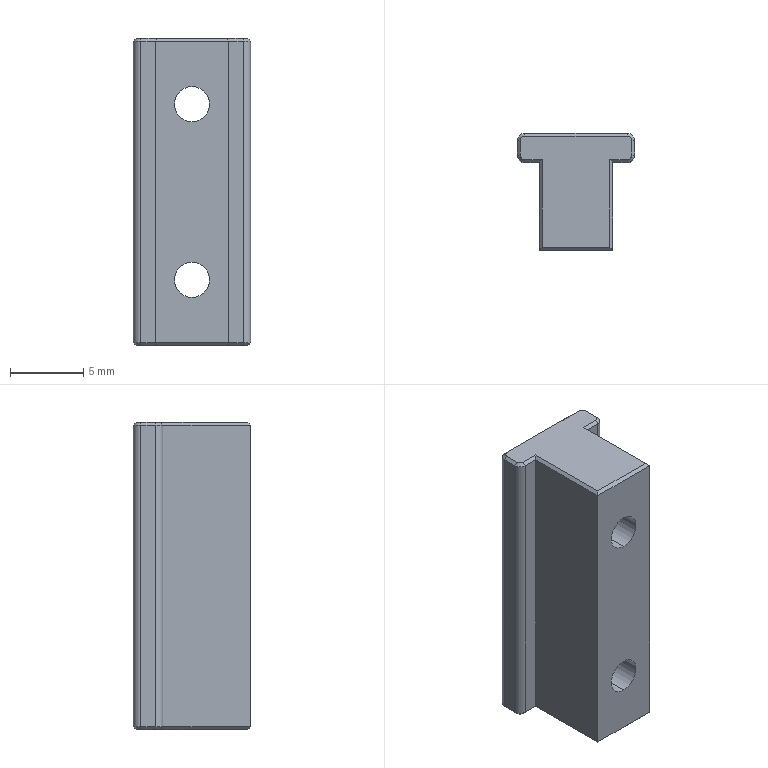Part | SolidWorks | features Fillet 2, ICE 2, Chamfer 1, Extrusion 1, HoleWzd 1 | 1 solid | 57 faces | box 8 x 8 x 21 mm | volume 820.469 mm3 | plane 33 | cylinder 16 | cone 8 | commonest cylinder face diameters 1 x8 2.4 x4 4.4 x4
STEP:
#1=CARTESIAN_POINT('',(0.,1.6,2.3));
#2=VERTEX_POINT('',#1);
#3=CARTESIAN_POINT('',(0.,1.6,6.7));
#4=VERTEX_POINT('',#3);
#5=CARTESIAN_POINT('',(0.,1.6,4.5));
#6=DIRECTION('',(0.,1.,0.));
#7=DIRECTION('',(0.,0.,1.));
#8=AXIS2_PLACEMENT_3D('',#5,#6,#7);
#9=CIRCLE('',#8,2.2);
#10=EDGE_CURVE('',#2,#4,#9,.T.);
#11=ORIENTED_EDGE('',*,*,#10,.F.);
#12=CARTESIAN_POINT('',(0.,4.,2.3));
#13=VERTEX_POINT('',#12);
#14=CARTESIAN_POINT('',(0.,4.,2.3));
#15=DIRECTION('',(0.,1.,0.));
#16=VECTOR('',#15,1000.);
#17=LINE('',#14,#16);
#18=EDGE_CURVE('',#2,#13,#17,.T.);
#19=ORIENTED_EDGE('',*,*,#18,.T.);
#20=CARTESIAN_POINT('',(0.,4.,6.7));
#21=VERTEX_POINT('',#20);
#22=CARTESIAN_POINT('',(0.,4.,4.5));
#23=DIRECTION('',(0.,1.,0.));
#24=DIRECTION('',(0.,0.,1.));
#25=AXIS2_PLACEMENT_3D('',#22,#23,#24);
#26=CIRCLE('',#25,2.2);
#27=EDGE_CURVE('',#13,#21,#26,.T.);
#28=ORIENTED_EDGE('',*,*,#27,.T.);
#29=CARTESIAN_POINT('',(0.,4.,6.7));
#30=DIRECTION('',(0.,1.,0.));
#31=VECTOR('',#30,1000.);
#32=LINE('',#29,#31);
#33=EDGE_CURVE('',#4,#21,#32,.T.);
#34=ORIENTED_EDGE('',*,*,#33,.F.);
#35=EDGE_LOOP('',(#11,#19,#28,#34));
#36=FACE_OUTER_BOUND('',#35,.T.);
#37=CARTESIAN_POINT('',(0.,4.,4.5));
#38=DIRECTION('',(0.,1.,0.));
#39=DIRECTION('',(0.,0.,1.));
#40=AXIS2_PLACEMENT_3D('',#37,#38,#39);
#41=CYLINDRICAL_SURFACE('',#40,2.2);
#42=ADVANCED_FACE('',(#36),#41,.F.);
#43=CARTESIAN_POINT('',(0.,-4.,3.3));
#44=VERTEX_POINT('',#43);
#45=CARTESIAN_POINT('',(0.,-4.,5.7));
#46=VERTEX_POINT('',#45);
#47=CARTESIAN_POINT('',(0.,-4.,4.5));
#48=DIRECTION('',(0.,1.,0.));
#49=DIRECTION('',(0.,0.,1.));
#50=AXIS2_PLACEMENT_3D('',#47,#48,#49);
#51=CIRCLE('',#50,1.2);
#52=EDGE_CURVE('',#44,#46,#51,.T.);
#53=ORIENTED_EDGE('',*,*,#52,.F.);
#54=CARTESIAN_POINT('',(0.,1.6,3.3));
#55=VERTEX_POINT('',#54);
#56=CARTESIAN_POINT('',(0.,4.,3.3));
#57=DIRECTION('',(0.,1.,0.));
#58=VECTOR('',#57,1000.);
#59=LINE('',#56,#58);
#60=EDGE_CURVE('',#44,#55,#59,.T.);
#61=ORIENTED_EDGE('',*,*,#60,.T.);
#62=CARTESIAN_POINT('',(0.,1.6,5.7));
#63=VERTEX_POINT('',#62);
#64=CARTESIAN_POINT('',(0.,1.6,4.5));
#65=DIRECTION('',(0.,1.,0.));
#66=DIRECTION('',(0.,0.,1.));
#67=AXIS2_PLACEMENT_3D('',#64,#65,#66);
#68=CIRCLE('',#67,1.2);
#69=EDGE_CURVE('',#55,#63,#68,.T.);
#70=ORIENTED_EDGE('',*,*,#69,.T.);
#71=CARTESIAN_POINT('',(0.,4.,5.7));
#72=DIRECTION('',(0.,1.,0.));
#73=VECTOR('',#72,1000.);
#74=LINE('',#71,#73);
#75=EDGE_CURVE('',#46,#63,#74,.T.);
#76=ORIENTED_EDGE('',*,*,#75,.F.);
#77=EDGE_LOOP('',(#53,#61,#70,#76));
#78=FACE_OUTER_BOUND('',#77,.T.);
#79=CARTESIAN_POINT('',(0.,4.,4.5));
#80=DIRECTION('',(0.,1.,0.));
#81=DIRECTION('',(0.,0.,1.));
#82=AXIS2_PLACEMENT_3D('',#79,#80,#81);
#83=CYLINDRICAL_SURFACE('',#82,1.2);
#84=ADVANCED_FACE('',(#78),#83,.F.);
#85=CARTESIAN_POINT('',(0.,1.6,14.3));
#86=VERTEX_POINT('',#85);
#87=CARTESIAN_POINT('',(0.,1.6,18.7));
#88=VERTEX_POINT('',#87);
#89=CARTESIAN_POINT('',(0.,1.6,16.5));
#90=DIRECTION('',(0.,1.,0.));
#91=DIRECTION('',(0.,0.,1.));
#92=AXIS2_PLACEMENT_3D('',#89,#90,#91);
#93=CIRCLE('',#92,2.2);
#94=EDGE_CURVE('',#86,#88,#93,.T.);
#95=ORIENTED_EDGE('',*,*,#94,.F.);
#96=CARTESIAN_POINT('',(0.,4.,14.3));
#97=VERTEX_POINT('',#96);
#98=CARTESIAN_POINT('',(0.,4.,14.3));
#99=DIRECTION('',(0.,1.,0.));
#100=VECTOR('',#99,1000.);
#101=LINE('',#98,#100);
#102=EDGE_CURVE('',#86,#97,#101,.T.);
#103=ORIENTED_EDGE('',*,*,#102,.T.);
#104=CARTESIAN_POINT('',(0.,4.,18.7));
#105=VERTEX_POINT('',#104);
#106=CARTESIAN_POINT('',(0.,4.,16.5));
#107=DIRECTION('',(0.,1.,0.));
#108=DIRECTION('',(0.,0.,1.));
#109=AXIS2_PLACEMENT_3D('',#106,#107,#108);
#110=CIRCLE('',#109,2.2);
#111=EDGE_CURVE('',#97,#105,#110,.T.);
#112=ORIENTED_EDGE('',*,*,#111,.T.);
#113=CARTESIAN_POINT('',(0.,4.,18.7));
#114=DIRECTION('',(0.,1.,0.));
#115=VECTOR('',#114,1000.);
#116=LINE('',#113,#115);
#117=EDGE_CURVE('',#88,#105,#116,.T.);
#118=ORIENTED_EDGE('',*,*,#117,.F.);
#119=EDGE_LOOP('',(#95,#103,#112,#118));
#120=FACE_OUTER_BOUND('',#119,.T.);
#121=CARTESIAN_POINT('',(0.,4.,16.5));
#122=DIRECTION('',(0.,1.,0.));
#123=DIRECTION('',(0.,0.,1.));
#124=AXIS2_PLACEMENT_3D('',#121,#122,#123);
#125=CYLINDRICAL_SURFACE('',#124,2.2);
#126=ADVANCED_FACE('',(#120),#125,.F.);
#127=CARTESIAN_POINT('',(0.,-4.,15.3));
#128=VERTEX_POINT('',#127);
#129=CARTESIAN_POINT('',(0.,-4.,17.7));
#130=VERTEX_POINT('',#129);
#131=CARTESIAN_POINT('',(0.,-4.,16.5));
#132=DIRECTION('',(0.,1.,0.));
#133=DIRECTION('',(0.,0.,1.));
#134=AXIS2_PLACEMENT_3D('',#131,#132,#133);
#135=CIRCLE('',#134,1.2);
#136=EDGE_CURVE('',#128,#130,#135,.T.);
#137=ORIENTED_EDGE('',*,*,#136,.F.);
#138=CARTESIAN_POINT('',(0.,1.6,15.3));
#139=VERTEX_POINT('',#138);
#140=CARTESIAN_POINT('',(0.,4.,15.3));
#141=DIRECTION('',(0.,1.,0.));
#142=VECTOR('',#141,1000.);
#143=LINE('',#140,#142);
#144=EDGE_CURVE('',#128,#139,#143,.T.);
#145=ORIENTED_EDGE('',*,*,#144,.T.);
#146=CARTESIAN_POINT('',(0.,1.6,17.7));
#147=VERTEX_POINT('',#146);
#148=CARTESIAN_POINT('',(0.,1.6,16.5));
#149=DIRECTION('',(0.,1.,0.));
#150=DIRECTION('',(0.,0.,1.));
#151=AXIS2_PLACEMENT_3D('',#148,#149,#150);
#152=CIRCLE('',#151,1.2);
#153=EDGE_CURVE('',#139,#147,#152,.T.);
#154=ORIENTED_EDGE('',*,*,#153,.T.);
#155=CARTESIAN_POINT('',(0.,4.,17.7));
#156=DIRECTION('',(0.,1.,0.));
#157=VECTOR('',#156,1000.);
#158=LINE('',#155,#157);
#159=EDGE_CURVE('',#130,#147,#158,.T.);
#160=ORIENTED_EDGE('',*,*,#159,.F.);
#161=EDGE_LOOP('',(#137,#145,#154,#160));
#162=FACE_OUTER_BOUND('',#161,.T.);
#163=CARTESIAN_POINT('',(0.,4.,16.5));
#164=DIRECTION('',(0.,1.,0.));
#165=DIRECTION('',(0.,0.,1.));
#166=AXIS2_PLACEMENT_3D('',#163,#164,#165);
#167=CYLINDRICAL_SURFACE('',#166,1.2);
#168=ADVANCED_FACE('',(#162),#167,.F.);
#169=CARTESIAN_POINT('',(4.,2.5,20.8));
#170=VERTEX_POINT('',#169);
#171=CARTESIAN_POINT('',(4.,2.5,0.2));
#172=VERTEX_POINT('',#171);
#173=CARTESIAN_POINT('',(4.,2.5,21.));
#174=DIRECTION('',(0.,0.,-1.));
#175=VECTOR('',#174,1000.);
#176=LINE('',#173,#175);
#177=EDGE_CURVE('',#170,#172,#176,.T.);
#178=ORIENTED_EDGE('',*,*,#177,.T.);
#179=CARTESIAN_POINT('',(4.,3.5,0.2));
#180=VERTEX_POINT('',#179);
#181=CARTESIAN_POINT('',(4.,4.,0.2));
#182=DIRECTION('',(0.,1.,0.));
#183=VECTOR('',#182,1000.);
#184=LINE('',#181,#183);
#185=EDGE_CURVE('',#172,#180,#184,.T.);
#186=ORIENTED_EDGE('',*,*,#185,.T.);
#187=CARTESIAN_POINT('',(4.,3.5,20.8));
#188=VERTEX_POINT('',#187);
#189=CARTESIAN_POINT('',(4.,3.5,21.));
#190=DIRECTION('',(0.,0.,1.));
#191=VECTOR('',#190,1000.);
#192=LINE('',#189,#191);
#193=EDGE_CURVE('',#180,#188,#192,.T.);
#194=ORIENTED_EDGE('',*,*,#193,.T.);
#195=CARTESIAN_POINT('',(4.,2.5,20.8));
#196=DIRECTION('',(0.,-1.,0.));
#197=VECTOR('',#196,1000.);
#198=LINE('',#195,#197);
#199=EDGE_CURVE('',#188,#170,#198,.T.);
#200=ORIENTED_EDGE('',*,*,#199,.T.);
#201=EDGE_LOOP('',(#178,#186,#194,#200));
#202=FACE_OUTER_BOUND('',#201,.T.);
#203=CARTESIAN_POINT('',(4.,4.,21.));
#204=DIRECTION('',(-1.,0.,0.));
#205=DIRECTION('',(0.,-1.,0.));
#206=AXIS2_PLACEMENT_3D('',#203,#204,#205);
#207=PLANE('',#206);
#208=ADVANCED_FACE('',(#202),#207,.F.);
#209=CARTESIAN_POINT('',(2.,4.,7.25));
#210=VERTEX_POINT('',#209);
#211=CARTESIAN_POINT('',(-2.,4.,7.25));
#212=VERTEX_POINT('',#211);
#213=CARTESIAN_POINT('',(-2.5,4.,7.25));
#214=DIRECTION('',(-1.,0.,0.));
#215=VECTOR('',#214,1000.);
#216=LINE('',#213,#215);
#217=EDGE_CURVE('',#210,#212,#216,.T.);
#218=ORIENTED_EDGE('',*,*,#217,.F.);
#219=CARTESIAN_POINT('',(2.5,4.,7.75));
#220=VERTEX_POINT('',#219);
#221=CARTESIAN_POINT('',(2.,4.,7.75));
#222=DIRECTION('',(0.,-1.,0.));
#223=DIRECTION('',(0.,0.,-1.));
#224=AXIS2_PLACEMENT_3D('',#221,#222,#223);
#225=CIRCLE('',#224,0.5);
#226=EDGE_CURVE('',#210,#220,#225,.T.);
#227=ORIENTED_EDGE('',*,*,#226,.T.);
#228=CARTESIAN_POINT('',(2.5,4.,13.25));
#229=VERTEX_POINT('',#228);
#230=CARTESIAN_POINT('',(2.5,4.,13.75));
#231=DIRECTION('',(0.,0.,-1.));
#232=VECTOR('',#231,1000.);
#233=LINE('',#230,#232);
#234=EDGE_CURVE('',#229,#220,#233,.T.);
#235=ORIENTED_EDGE('',*,*,#234,.F.);
#236=CARTESIAN_POINT('',(2.,4.,13.75));
#237=VERTEX_POINT('',#236);
#238=CARTESIAN_POINT('',(2.,4.,13.25));
#239=DIRECTION('',(0.,-1.,0.));
#240=DIRECTION('',(0.,0.,-1.));
#241=AXIS2_PLACEMENT_3D('',#238,#239,#240);
#242=CIRCLE('',#241,0.5);
#243=EDGE_CURVE('',#229,#237,#242,.T.);
#244=ORIENTED_EDGE('',*,*,#243,.T.);
#245=CARTESIAN_POINT('',(-2.,4.,13.75));
#246=VERTEX_POINT('',#245);
#247=CARTESIAN_POINT('',(-2.5,4.,13.75));
#248=DIRECTION('',(1.,0.,0.));
#249=VECTOR('',#248,1000.);
#250=LINE('',#247,#249);
#251=EDGE_CURVE('',#246,#237,#250,.T.);
#252=ORIENTED_EDGE('',*,*,#251,.F.);
#253=CARTESIAN_POINT('',(-2.5,4.,13.25));
#254=VERTEX_POINT('',#253);
#255=CARTESIAN_POINT('',(-2.,4.,13.25));
#256=DIRECTION('',(0.,-1.,0.));
#257=DIRECTION('',(0.,0.,-1.));
#258=AXIS2_PLACEMENT_3D('',#255,#256,#257);
#259=CIRCLE('',#258,0.5);
#260=EDGE_CURVE('',#246,#254,#259,.T.);
#261=ORIENTED_EDGE('',*,*,#260,.T.);
#262=CARTESIAN_POINT('',(-2.5,4.,7.75));
#263=VERTEX_POINT('',#262);
#264=CARTESIAN_POINT('',(-2.5,4.,13.75));
#265=DIRECTION('',(0.,0.,1.));
#266=VECTOR('',#265,1000.);
#267=LINE('',#264,#266);
#268=EDGE_CURVE('',#263,#254,#267,.T.);
#269=ORIENTED_EDGE('',*,*,#268,.F.);
#270=CARTESIAN_POINT('',(-2.,4.,7.75));
#271=DIRECTION('',(0.,-1.,0.));
#272=DIRECTION('',(0.,0.,-1.));
#273=AXIS2_PLACEMENT_3D('',#270,#271,#272);
#274=CIRCLE('',#273,0.5);
#275=EDGE_CURVE('',#263,#212,#274,.T.);
#276=ORIENTED_EDGE('',*,*,#275,.T.);
#277=EDGE_LOOP('',(#218,#227,#235,#244,#252,#261,#269,#276));
#278=FACE_BOUND('',#277,.T.);
#279=CARTESIAN_POINT('',(0.,4.,4.5));
#280=DIRECTION('',(0.,1.,0.));
#281=DIRECTION('',(0.,0.,1.));
#282=AXIS2_PLACEMENT_3D('',#279,#280,#281);
#283=CIRCLE('',#282,2.2);
#284=EDGE_CURVE('',#21,#13,#283,.T.);
#285=ORIENTED_EDGE('',*,*,#284,.F.);
#286=ORIENTED_EDGE('',*,*,#27,.F.);
#287=EDGE_LOOP('',(#285,#286));
#288=FACE_BOUND('',#287,.T.);
#289=CARTESIAN_POINT('',(0.,4.,16.5));
#290=DIRECTION('',(0.,1.,0.));
#291=DIRECTION('',(0.,0.,1.));
#292=AXIS2_PLACEMENT_3D('',#289,#290,#291);
#293=CIRCLE('',#292,2.2);
#294=EDGE_CURVE('',#105,#97,#293,.T.);
#295=ORIENTED_EDGE('',*,*,#294,.F.);
#296=ORIENTED_EDGE('',*,*,#111,.F.);
#297=EDGE_LOOP('',(#295,#296));
#298=FACE_BOUND('',#297,.T.);
#299=CARTESIAN_POINT('',(3.5,4.,20.8));
#300=VERTEX_POINT('',#299);
#301=CARTESIAN_POINT('',(3.5,4.,0.2));
#302=VERTEX_POINT('',#301);
#303=CARTESIAN_POINT('',(3.5,4.,21.));
#304=DIRECTION('',(0.,0.,-1.));
#305=VECTOR('',#304,1000.);
#306=LINE('',#303,#305);
#307=EDGE_CURVE('',#300,#302,#306,.T.);
#308=ORIENTED_EDGE('',*,*,#307,.T.);
#309=CARTESIAN_POINT('',(-3.5,4.,0.2));
#310=VERTEX_POINT('',#309);
#311=CARTESIAN_POINT('',(-4.,4.,0.2));
#312=DIRECTION('',(-1.,0.,0.));
#313=VECTOR('',#312,1000.);
#314=LINE('',#311,#313);
#315=EDGE_CURVE('',#302,#310,#314,.T.);
#316=ORIENTED_EDGE('',*,*,#315,.T.);
#317=CARTESIAN_POINT('',(-3.5,4.,20.8));
#318=VERTEX_POINT('',#317);
#319=CARTESIAN_POINT('',(-3.5,4.,21.));
#320=DIRECTION('',(0.,0.,1.));
#321=VECTOR('',#320,1000.);
#322=LINE('',#319,#321);
#323=EDGE_CURVE('',#310,#318,#322,.T.);
#324=ORIENTED_EDGE('',*,*,#323,.T.);
#325=CARTESIAN_POINT('',(3.5,4.,20.8));
#326=DIRECTION('',(1.,0.,0.));
#327=VECTOR('',#326,1000.);
#328=LINE('',#325,#327);
#329=EDGE_CURVE('',#318,#300,#328,.T.);
#330=ORIENTED_EDGE('',*,*,#329,.T.);
#331=EDGE_LOOP('',(#308,#316,#324,#330));
#332=FACE_OUTER_BOUND('',#331,.T.);
#333=CARTESIAN_POINT('',(-4.,4.,21.));
#334=DIRECTION('',(0.,-1.,0.));
#335=DIRECTION('',(0.,0.,-1.));
#336=AXIS2_PLACEMENT_3D('',#333,#334,#335);
#337=PLANE('',#336);
#338=ADVANCED_FACE('',(#278,#288,#298,#332),#337,.F.);
#339=CARTESIAN_POINT('',(-4.,3.5,20.8));
#340=VERTEX_POINT('',#339);
#341=CARTESIAN_POINT('',(-4.,3.5,0.2));
#342=VERTEX_POINT('',#341);
#343=CARTESIAN_POINT('',(-4.,3.5,21.));
#344=DIRECTION('',(0.,0.,-1.));
#345=VECTOR('',#344,1000.);
#346=LINE('',#343,#345);
#347=EDGE_CURVE('',#340,#342,#346,.T.);
#348=ORIENTED_EDGE('',*,*,#347,.T.);
#349=CARTESIAN_POINT('',(-4.,2.5,0.2));
#350=VERTEX_POINT('',#349);
#351=CARTESIAN_POINT('',(-4.,4.,0.2));
#352=DIRECTION('',(0.,-1.,0.));
#353=VECTOR('',#352,1000.);
#354=LINE('',#351,#353);
#355=EDGE_CURVE('',#342,#350,#354,.T.);
#356=ORIENTED_EDGE('',*,*,#355,.T.);
#357=CARTESIAN_POINT('',(-4.,2.5,20.8));
#358=VERTEX_POINT('',#357);
#359=CARTESIAN_POINT('',(-4.,2.5,21.));
#360=DIRECTION('',(0.,0.,1.));
#361=VECTOR('',#360,1000.);
#362=LINE('',#359,#361);
#363=EDGE_CURVE('',#350,#358,#362,.T.);
#364=ORIENTED_EDGE('',*,*,#363,.T.);
#365=CARTESIAN_POINT('',(-4.,3.5,20.8));
#366=DIRECTION('',(0.,1.,0.));
#367=VECTOR('',#366,1000.);
#368=LINE('',#365,#367);
#369=EDGE_CURVE('',#358,#340,#368,.T.);
#370=ORIENTED_EDGE('',*,*,#369,.T.);
#371=EDGE_LOOP('',(#348,#356,#364,#370));
#372=FACE_OUTER_BOUND('',#371,.T.);
#373=CARTESIAN_POINT('',(-4.,4.,21.));
#374=DIRECTION('',(1.,0.,0.));
#375=DIRECTION('',(0.,1.,0.));
#376=AXIS2_PLACEMENT_3D('',#373,#374,#375);
#377=PLANE('',#376);
#378=ADVANCED_FACE('',(#372),#377,.F.);
#379=CARTESIAN_POINT('',(0.,-4.,4.5));
#380=DIRECTION('',(0.,1.,0.));
#381=DIRECTION('',(0.,0.,1.));
#382=AXIS2_PLACEMENT_3D('',#379,#380,#381);
#383=CIRCLE('',#382,1.2);
#384=EDGE_CURVE('',#46,#44,#383,.T.);
#385=ORIENTED_EDGE('',*,*,#384,.T.);
#386=ORIENTED_EDGE('',*,*,#52,.T.);
#387=EDGE_LOOP('',(#385,#386));
#388=FACE_BOUND('',#387,.T.);
#389=CARTESIAN_POINT('',(0.,-4.,16.5));
#390=DIRECTION('',(0.,1.,0.));
#391=DIRECTION('',(0.,0.,1.));
#392=AXIS2_PLACEMENT_3D('',#389,#390,#391);
#393=CIRCLE('',#392,1.2);
#394=EDGE_CURVE('',#130,#128,#393,.T.);
#395=ORIENTED_EDGE('',*,*,#394,.T.);
#396=ORIENTED_EDGE('',*,*,#136,.T.);
#397=EDGE_LOOP('',(#395,#396));
#398=FACE_BOUND('',#397,.T.);
#399=CARTESIAN_POINT('',(-2.5,-4.,0.2));
#400=VERTEX_POINT('',#399);
#401=CARTESIAN_POINT('',(-2.5,-4.,20.8));
#402=VERTEX_POINT('',#401);
#403=CARTESIAN_POINT('',(-2.5,-4.,0.));
#404=DIRECTION('',(0.,0.,1.));
#405=VECTOR('',#404,1000.);
#406=LINE('',#403,#405);
#407=EDGE_CURVE('',#400,#402,#406,.T.);
#408=ORIENTED_EDGE('',*,*,#407,.F.);
#409=CARTESIAN_POINT('',(2.5,-4.,0.2));
#410=VERTEX_POINT('',#409);
#411=CARTESIAN_POINT('',(-4.,-4.,0.2));
#412=DIRECTION('',(1.,0.,0.));
#413=VECTOR('',#412,1000.);
#414=LINE('',#411,#413);
#415=EDGE_CURVE('',#400,#410,#414,.T.);
#416=ORIENTED_EDGE('',*,*,#415,.T.);
#417=CARTESIAN_POINT('',(2.5,-4.,20.8));
#418=VERTEX_POINT('',#417);
#419=CARTESIAN_POINT('',(2.5,-4.,0.));
#420=DIRECTION('',(0.,0.,1.));
#421=VECTOR('',#420,1000.);
#422=LINE('',#419,#421);
#423=EDGE_CURVE('',#410,#418,#422,.T.);
#424=ORIENTED_EDGE('',*,*,#423,.T.);
#425=CARTESIAN_POINT('',(-2.5,-4.,20.8));
#426=DIRECTION('',(-1.,0.,0.));
#427=VECTOR('',#426,1000.);
#428=LINE('',#425,#427);
#429=EDGE_CURVE('',#418,#402,#428,.T.);
#430=ORIENTED_EDGE('',*,*,#429,.T.);
#431=EDGE_LOOP('',(#408,#416,#424,#430));
#432=FACE_OUTER_BOUND('',#431,.T.);
#433=CARTESIAN_POINT('',(-4.,-4.,21.));
#434=DIRECTION('',(0.,1.,0.));
#435=DIRECTION('',(0.,0.,1.));
#436=AXIS2_PLACEMENT_3D('',#433,#434,#435);
#437=PLANE('',#436);
#438=ADVANCED_FACE('',(#388,#398,#432),#437,.F.);
#439=CARTESIAN_POINT('',(2.3,2.2,21.));
#440=VERTEX_POINT('',#439);
#441=CARTESIAN_POINT('',(3.5,2.2,21.));
#442=VERTEX_POINT('',#441);
#443=CARTESIAN_POINT('',(3.5,2.2,21.));
#444=DIRECTION('',(1.,0.,0.));
#445=VECTOR('',#444,1000.);
#446=LINE('',#443,#445);
#447=EDGE_CURVE('',#440,#442,#446,.T.);
#448=ORIENTED_EDGE('',*,*,#447,.T.);
#449=CARTESIAN_POINT('',(3.8,2.5,21.));
#450=VERTEX_POINT('',#449);
#451=CARTESIAN_POINT('',(3.5,2.5,21.));
#452=DIRECTION('',(0.,0.,1.));
#453=DIRECTION('',(1.,0.,0.));
#454=AXIS2_PLACEMENT_3D('',#451,#452,#453);
#455=CIRCLE('',#454,0.3);
#456=EDGE_CURVE('',#442,#450,#455,.T.);
#457=ORIENTED_EDGE('',*,*,#456,.T.);
#458=CARTESIAN_POINT('',(3.8,3.5,21.));
#459=VERTEX_POINT('',#458);
#460=CARTESIAN_POINT('',(3.8,3.5,21.));
#461=DIRECTION('',(0.,1.,0.));
#462=VECTOR('',#461,1000.);
#463=LINE('',#460,#462);
#464=EDGE_CURVE('',#450,#459,#463,.T.);
#465=ORIENTED_EDGE('',*,*,#464,.T.);
#466=CARTESIAN_POINT('',(3.5,3.8,21.));
#467=VERTEX_POINT('',#466);
#468=CARTESIAN_POINT('',(3.5,3.5,21.));
#469=DIRECTION('',(0.,0.,1.));
#470=DIRECTION('',(1.,0.,0.));
#471=AXIS2_PLACEMENT_3D('',#468,#469,#470);
#472=CIRCLE('',#471,0.3);
#473=EDGE_CURVE('',#459,#467,#472,.T.);
#474=ORIENTED_EDGE('',*,*,#473,.T.);
#475=CARTESIAN_POINT('',(-3.5,3.8,21.));
#476=VERTEX_POINT('',#475);
#477=CARTESIAN_POINT('',(-3.5,3.8,21.));
#478=DIRECTION('',(-1.,0.,0.));
#479=VECTOR('',#478,1000.);
#480=LINE('',#477,#479);
#481=EDGE_CURVE('',#467,#476,#480,.T.);
#482=ORIENTED_EDGE('',*,*,#481,.T.);
#483=CARTESIAN_POINT('',(-3.8,3.5,21.));
#484=VERTEX_POINT('',#483);
#485=CARTESIAN_POINT('',(-3.5,3.5,21.));
#486=DIRECTION('',(0.,0.,1.));
#487=DIRECTION('',(1.,0.,0.));
#488=AXIS2_PLACEMENT_3D('',#485,#486,#487);
#489=CIRCLE('',#488,0.3);
#490=EDGE_CURVE('',#476,#484,#489,.T.);
#491=ORIENTED_EDGE('',*,*,#490,.T.);
#492=CARTESIAN_POINT('',(-3.8,2.5,21.));
#493=VERTEX_POINT('',#492);
#494=CARTESIAN_POINT('',(-3.8,2.5,21.));
#495=DIRECTION('',(0.,-1.,0.));
#496=VECTOR('',#495,1000.);
#497=LINE('',#494,#496);
#498=EDGE_CURVE('',#484,#493,#497,.T.);
#499=ORIENTED_EDGE('',*,*,#498,.T.);
#500=CARTESIAN_POINT('',(-3.5,2.2,21.));
#501=VERTEX_POINT('',#500);
#502=CARTESIAN_POINT('',(-3.5,2.5,21.));
#503=DIRECTION('',(0.,0.,1.));
#504=DIRECTION('',(1.,0.,0.));
#505=AXIS2_PLACEMENT_3D('',#502,#503,#504);
#506=CIRCLE('',#505,0.3);
#507=EDGE_CURVE('',#493,#501,#506,.T.);
#508=ORIENTED_EDGE('',*,*,#507,.T.);
#509=CARTESIAN_POINT('',(-2.3,2.2,21.));
#510=VERTEX_POINT('',#509);
#511=CARTESIAN_POINT('',(-2.5,2.2,21.));
#512=DIRECTION('',(1.,0.,0.));
#513=VECTOR('',#512,1000.);
#514=LINE('',#511,#513);
#515=EDGE_CURVE('',#501,#510,#514,.T.);
#516=ORIENTED_EDGE('',*,*,#515,.T.);
#517=CARTESIAN_POINT('',(-2.3,-3.8,21.));
#518=VERTEX_POINT('',#517);
#519=CARTESIAN_POINT('',(-2.3,-4.,21.));
#520=DIRECTION('',(0.,-1.,0.));
#521=VECTOR('',#520,1000.);
#522=LINE('',#519,#521);
#523=EDGE_CURVE('',#510,#518,#522,.T.);
#524=ORIENTED_EDGE('',*,*,#523,.T.);
#525=CARTESIAN_POINT('',(2.3,-3.8,21.));
#526=VERTEX_POINT('',#525);
#527=CARTESIAN_POINT('',(2.5,-3.8,21.));
#528=DIRECTION('',(1.,0.,0.));
#529=VECTOR('',#528,1000.);
#530=LINE('',#527,#529);
#531=EDGE_CURVE('',#518,#526,#530,.T.);
#532=ORIENTED_EDGE('',*,*,#531,.T.);
#533=CARTESIAN_POINT('',(2.3,2.,21.));
#534=DIRECTION('',(0.,1.,0.));
#535=VECTOR('',#534,1000.);
#536=LINE('',#533,#535);
#537=EDGE_CURVE('',#526,#440,#536,.T.);
#538=ORIENTED_EDGE('',*,*,#537,.T.);
#539=EDGE_LOOP('',(#448,#457,#465,#474,#482,#491,#499,#508,#516,#524,#532,#538));
#540=FACE_OUTER_BOUND('',#539,.T.);
#541=CARTESIAN_POINT('',(0.,0.,21.));
#542=DIRECTION('',(0.,0.,1.));
#543=DIRECTION('',(1.,0.,0.));
#544=AXIS2_PLACEMENT_3D('',#541,#542,#543);
#545=PLANE('',#544);
#546=ADVANCED_FACE('',(#540),#545,.T.);
#547=CARTESIAN_POINT('',(-3.8,2.5,0.));
#548=VERTEX_POINT('',#547);
#549=CARTESIAN_POINT('',(-3.8,3.5,0.));
#550=VERTEX_POINT('',#549);
#551=CARTESIAN_POINT('',(-3.8,0.,0.));
#552=DIRECTION('',(0.,1.,0.));
#553=VECTOR('',#552,1000.);
#554=LINE('',#551,#553);
#555=EDGE_CURVE('',#548,#550,#554,.T.);
#556=ORIENTED_EDGE('',*,*,#555,.T.);
#557=CARTESIAN_POINT('',(-3.5,3.8,0.));
#558=VERTEX_POINT('',#557);
#559=CARTESIAN_POINT('',(-3.5,3.5,0.));
#560=DIRECTION('',(0.,0.,-1.));
#561=DIRECTION('',(1.,0.,0.));
#562=AXIS2_PLACEMENT_3D('',#559,#560,#561);
#563=CIRCLE('',#562,0.3);
#564=EDGE_CURVE('',#550,#558,#563,.T.);
#565=ORIENTED_EDGE('',*,*,#564,.T.);
#566=CARTESIAN_POINT('',(3.5,3.8,0.));
#567=VERTEX_POINT('',#566);
#568=CARTESIAN_POINT('',(0.,3.8,0.));
#569=DIRECTION('',(1.,0.,0.));
#570=VECTOR('',#569,1000.);
#571=LINE('',#568,#570);
#572=EDGE_CURVE('',#558,#567,#571,.T.);
#573=ORIENTED_EDGE('',*,*,#572,.T.);
#574=CARTESIAN_POINT('',(3.8,3.5,0.));
#575=VERTEX_POINT('',#574);
#576=CARTESIAN_POINT('',(3.5,3.5,0.));
#577=DIRECTION('',(0.,0.,-1.));
#578=DIRECTION('',(1.,0.,0.));
#579=AXIS2_PLACEMENT_3D('',#576,#577,#578);
#580=CIRCLE('',#579,0.3);
#581=EDGE_CURVE('',#567,#575,#580,.T.);
#582=ORIENTED_EDGE('',*,*,#581,.T.);
#583=CARTESIAN_POINT('',(3.8,2.5,0.));
#584=VERTEX_POINT('',#583);
#585=CARTESIAN_POINT('',(3.8,0.,0.));
#586=DIRECTION('',(0.,-1.,0.));
#587=VECTOR('',#586,1000.);
#588=LINE('',#585,#587);
#589=EDGE_CURVE('',#575,#584,#588,.T.);
#590=ORIENTED_EDGE('',*,*,#589,.T.);
#591=CARTESIAN_POINT('',(3.5,2.2,0.));
#592=VERTEX_POINT('',#591);
#593=CARTESIAN_POINT('',(3.5,2.5,0.));
#594=DIRECTION('',(0.,0.,-1.));
#595=DIRECTION('',(1.,0.,0.));
#596=AXIS2_PLACEMENT_3D('',#593,#594,#595);
#597=CIRCLE('',#596,0.3);
#598=EDGE_CURVE('',#584,#592,#597,.T.);
#599=ORIENTED_EDGE('',*,*,#598,.T.);
#600=CARTESIAN_POINT('',(2.3,2.2,0.));
#601=VERTEX_POINT('',#600);
#602=CARTESIAN_POINT('',(0.,2.2,0.));
#603=DIRECTION('',(-1.,0.,0.));
#604=VECTOR('',#603,1000.);
#605=LINE('',#602,#604);
#606=EDGE_CURVE('',#592,#601,#605,.T.);
#607=ORIENTED_EDGE('',*,*,#606,.T.);
#608=CARTESIAN_POINT('',(2.3,-3.8,0.));
#609=VERTEX_POINT('',#608);
#610=CARTESIAN_POINT('',(2.3,0.,0.));
#611=DIRECTION('',(0.,-1.,0.));
#612=VECTOR('',#611,1000.);
#613=LINE('',#610,#612);
#614=EDGE_CURVE('',#601,#609,#613,.T.);
#615=ORIENTED_EDGE('',*,*,#614,.T.);
#616=CARTESIAN_POINT('',(-2.3,-3.8,0.));
#617=VERTEX_POINT('',#616);
#618=CARTESIAN_POINT('',(0.,-3.8,0.));
#619=DIRECTION('',(-1.,0.,0.));
#620=VECTOR('',#619,1000.);
#621=LINE('',#618,#620);
#622=EDGE_CURVE('',#609,#617,#621,.T.);
#623=ORIENTED_EDGE('',*,*,#622,.T.);
#624=CARTESIAN_POINT('',(-2.3,2.2,0.));
#625=VERTEX_POINT('',#624);
#626=CARTESIAN_POINT('',(-2.3,0.,0.));
#627=DIRECTION('',(0.,1.,0.));
#628=VECTOR('',#627,1000.);
#629=LINE('',#626,#628);
#630=EDGE_CURVE('',#617,#625,#629,.T.);
#631=ORIENTED_EDGE('',*,*,#630,.T.);
#632=CARTESIAN_POINT('',(-3.5,2.2,0.));
#633=VERTEX_POINT('',#632);
#634=CARTESIAN_POINT('',(0.,2.2,0.));
#635=DIRECTION('',(-1.,0.,0.));
#636=VECTOR('',#635,1000.);
#637=LINE('',#634,#636);
#638=EDGE_CURVE('',#625,#633,#637,.T.);
#639=ORIENTED_EDGE('',*,*,#638,.T.);
#640=CARTESIAN_POINT('',(-3.5,2.5,0.));
#641=DIRECTION('',(0.,0.,-1.));
#642=DIRECTION('',(1.,0.,0.));
#643=AXIS2_PLACEMENT_3D('',#640,#641,#642);
#644=CIRCLE('',#643,0.3);
#645=EDGE_CURVE('',#633,#548,#644,.T.);
#646=ORIENTED_EDGE('',*,*,#645,.T.);
#647=EDGE_LOOP('',(#556,#565,#573,#582,#590,#599,#607,#615,#623,#631,#639,#646));
#648=FACE_OUTER_BOUND('',#647,.T.);
#649=CARTESIAN_POINT('',(0.,0.,0.));
#650=DIRECTION('',(0.,0.,1.));
#651=DIRECTION('',(1.,0.,0.));
#652=AXIS2_PLACEMENT_3D('',#649,#650,#651);
#653=PLANE('',#652);
#654=ADVANCED_FACE('',(#648),#653,.F.);
#655=ORIENTED_EDGE('',*,*,#423,.F.);
#656=CARTESIAN_POINT('',(2.5,2.,0.2));
#657=VERTEX_POINT('',#656);
#658=CARTESIAN_POINT('',(2.5,-4.,0.2));
#659=DIRECTION('',(0.,1.,0.));
#660=VECTOR('',#659,1000.);
#661=LINE('',#658,#660);
#662=EDGE_CURVE('',#410,#657,#661,.T.);
#663=ORIENTED_EDGE('',*,*,#662,.T.);
#664=CARTESIAN_POINT('',(2.5,2.,20.8));
#665=VERTEX_POINT('',#664);
#666=CARTESIAN_POINT('',(2.5,2.,0.));
#667=DIRECTION('',(0.,0.,1.));
#668=VECTOR('',#667,1000.);
#669=LINE('',#666,#668);
#670=EDGE_CURVE('',#657,#665,#669,.T.);
#671=ORIENTED_EDGE('',*,*,#670,.T.);
#672=CARTESIAN_POINT('',(2.5,-4.,20.8));
#673=DIRECTION('',(0.,-1.,0.));
#674=VECTOR('',#673,1000.);
#675=LINE('',#672,#674);
#676=EDGE_CURVE('',#665,#418,#675,.T.);
#677=ORIENTED_EDGE('',*,*,#676,.T.);
#678=EDGE_LOOP('',(#655,#663,#671,#677));
#679=FACE_OUTER_BOUND('',#678,.T.);
#680=CARTESIAN_POINT('',(2.5,-4.,0.));
#681=DIRECTION('',(-1.,0.,0.));
#682=DIRECTION('',(0.,-1.,0.));
#683=AXIS2_PLACEMENT_3D('',#680,#681,#682);
#684=PLANE('',#683);
#685=ADVANCED_FACE('',(#679),#684,.F.);
#686=ORIENTED_EDGE('',*,*,#670,.F.);
#687=CARTESIAN_POINT('',(3.5,2.,0.2));
#688=VERTEX_POINT('',#687);
#689=CARTESIAN_POINT('',(4.,2.,0.2));
#690=DIRECTION('',(1.,0.,0.));
#691=VECTOR('',#690,1000.);
#692=LINE('',#689,#691);
#693=EDGE_CURVE('',#657,#688,#692,.T.);
#694=ORIENTED_EDGE('',*,*,#693,.T.);
#695=CARTESIAN_POINT('',(3.5,2.,20.8));
#696=VERTEX_POINT('',#695);
#697=CARTESIAN_POINT('',(3.5,2.,0.));
#698=DIRECTION('',(0.,0.,1.));
#699=VECTOR('',#698,1000.);
#700=LINE('',#697,#699);
#701=EDGE_CURVE('',#688,#696,#700,.T.);
#702=ORIENTED_EDGE('',*,*,#701,.T.);
#703=CARTESIAN_POINT('',(2.5,2.,20.8));
#704=DIRECTION('',(-1.,0.,0.));
#705=VECTOR('',#704,1000.);
#706=LINE('',#703,#705);
#707=EDGE_CURVE('',#696,#665,#706,.T.);
#708=ORIENTED_EDGE('',*,*,#707,.T.);
#709=EDGE_LOOP('',(#686,#694,#702,#708));
#710=FACE_OUTER_BOUND('',#709,.T.);
#711=CARTESIAN_POINT('',(4.,2.,0.));
#712=DIRECTION('',(0.,1.,0.));
#713=DIRECTION('',(-1.,0.,0.));
#714=AXIS2_PLACEMENT_3D('',#711,#712,#713);
#715=PLANE('',#714);
#716=ADVANCED_FACE('',(#710),#715,.F.);
#717=CARTESIAN_POINT('',(-3.5,2.,20.8));
#718=VERTEX_POINT('',#717);
#719=CARTESIAN_POINT('',(-3.5,2.,0.2));
#720=VERTEX_POINT('',#719);
#721=CARTESIAN_POINT('',(-3.5,2.,0.));
#722=DIRECTION('',(0.,0.,-1.));
#723=VECTOR('',#722,1000.);
#724=LINE('',#721,#723);
#725=EDGE_CURVE('',#718,#720,#724,.T.);
#726=ORIENTED_EDGE('',*,*,#725,.T.);
#727=CARTESIAN_POINT('',(-2.5,2.,0.2));
#728=VERTEX_POINT('',#727);
#729=CARTESIAN_POINT('',(-4.,2.,0.2));
#730=DIRECTION('',(1.,0.,0.));
#731=VECTOR('',#730,1000.);
#732=LINE('',#729,#731);
#733=EDGE_CURVE('',#720,#728,#732,.T.);
#734=ORIENTED_EDGE('',*,*,#733,.T.);
#735=CARTESIAN_POINT('',(-2.5,2.,20.8));
#736=VERTEX_POINT('',#735);
#737=CARTESIAN_POINT('',(-2.5,2.,0.));
#738=DIRECTION('',(0.,0.,1.));
#739=VECTOR('',#738,1000.);
#740=LINE('',#737,#739);
#741=EDGE_CURVE('',#728,#736,#740,.T.);
#742=ORIENTED_EDGE('',*,*,#741,.T.);
#743=CARTESIAN_POINT('',(-3.5,2.,20.8));
#744=DIRECTION('',(-1.,0.,0.));
#745=VECTOR('',#744,1000.);
#746=LINE('',#743,#745);
#747=EDGE_CURVE('',#736,#718,#746,.T.);
#748=ORIENTED_EDGE('',*,*,#747,.T.);
#749=EDGE_LOOP('',(#726,#734,#742,#748));
#750=FACE_OUTER_BOUND('',#749,.T.);
#751=CARTESIAN_POINT('',(-4.,2.,0.));
#752=DIRECTION('',(0.,1.,0.));
#753=DIRECTION('',(-1.,0.,0.));
#754=AXIS2_PLACEMENT_3D('',#751,#752,#753);
#755=PLANE('',#754);
#756=ADVANCED_FACE('',(#750),#755,.F.);
#757=ORIENTED_EDGE('',*,*,#741,.F.);
#758=CARTESIAN_POINT('',(-2.5,-4.,0.2));
#759=DIRECTION('',(0.,-1.,0.));
#760=VECTOR('',#759,1000.);
#761=LINE('',#758,#760);
#762=EDGE_CURVE('',#728,#400,#761,.T.);
#763=ORIENTED_EDGE('',*,*,#762,.T.);
#764=ORIENTED_EDGE('',*,*,#407,.T.);
#765=CARTESIAN_POINT('',(-2.5,2.,20.8));
#766=DIRECTION('',(0.,1.,0.));
#767=VECTOR('',#766,1000.);
#768=LINE('',#765,#767);
#769=EDGE_CURVE('',#402,#736,#768,.T.);
#770=ORIENTED_EDGE('',*,*,#769,.T.);
#771=EDGE_LOOP('',(#757,#763,#764,#770));
#772=FACE_OUTER_BOUND('',#771,.T.);
#773=CARTESIAN_POINT('',(-2.5,-4.,0.));
#774=DIRECTION('',(1.,0.,0.));
#775=DIRECTION('',(0.,0.,-1.));
#776=AXIS2_PLACEMENT_3D('',#773,#774,#775);
#777=PLANE('',#776);
#778=ADVANCED_FACE('',(#772),#777,.F.);
#779=ORIENTED_EDGE('',*,*,#193,.F.);
#780=CARTESIAN_POINT('',(3.5,3.5,0.2));
#781=DIRECTION('',(0.,0.,1.));
#782=DIRECTION('',(1.,0.,0.));
#783=AXIS2_PLACEMENT_3D('',#780,#781,#782);
#784=CIRCLE('',#783,0.5);
#785=EDGE_CURVE('',#180,#302,#784,.T.);
#786=ORIENTED_EDGE('',*,*,#785,.T.);
#787=ORIENTED_EDGE('',*,*,#307,.F.);
#788=CARTESIAN_POINT('',(3.5,3.5,20.8));
#789=DIRECTION('',(0.,0.,-1.));
#790=DIRECTION('',(1.,0.,0.));
#791=AXIS2_PLACEMENT_3D('',#788,#789,#790);
#792=CIRCLE('',#791,0.5);
#793=EDGE_CURVE('',#300,#188,#792,.T.);
#794=ORIENTED_EDGE('',*,*,#793,.T.);
#795=EDGE_LOOP('',(#779,#786,#787,#794));
#796=FACE_OUTER_BOUND('',#795,.T.);
#797=CARTESIAN_POINT('',(3.5,3.5,21.));
#798=DIRECTION('',(0.,0.,-1.));
#799=DIRECTION('',(-1.,0.,0.));
#800=AXIS2_PLACEMENT_3D('',#797,#798,#799);
#801=CYLINDRICAL_SURFACE('',#800,0.5);
#802=ADVANCED_FACE('',(#796),#801,.T.);
#803=ORIENTED_EDGE('',*,*,#701,.F.);
#804=CARTESIAN_POINT('',(3.5,2.5,0.2));
#805=DIRECTION('',(0.,0.,1.));
#806=DIRECTION('',(1.,0.,0.));
#807=AXIS2_PLACEMENT_3D('',#804,#805,#806);
#808=CIRCLE('',#807,0.5);
#809=EDGE_CURVE('',#688,#172,#808,.T.);
#810=ORIENTED_EDGE('',*,*,#809,.T.);
#811=ORIENTED_EDGE('',*,*,#177,.F.);
#812=CARTESIAN_POINT('',(3.5,2.5,20.8));
#813=DIRECTION('',(0.,0.,-1.));
#814=DIRECTION('',(1.,0.,0.));
#815=AXIS2_PLACEMENT_3D('',#812,#813,#814);
#816=CIRCLE('',#815,0.5);
#817=EDGE_CURVE('',#170,#696,#816,.T.);
#818=ORIENTED_EDGE('',*,*,#817,.T.);
#819=EDGE_LOOP('',(#803,#810,#811,#818));
#820=FACE_OUTER_BOUND('',#819,.T.);
#821=CARTESIAN_POINT('',(3.5,2.5,0.));
#822=DIRECTION('',(0.,0.,1.));
#823=DIRECTION('',(1.,0.,0.));
#824=AXIS2_PLACEMENT_3D('',#821,#822,#823);
#825=CYLINDRICAL_SURFACE('',#824,0.5);
#826=ADVANCED_FACE('',(#820),#825,.T.);
#827=ORIENTED_EDGE('',*,*,#323,.F.);
#828=CARTESIAN_POINT('',(-3.5,3.5,0.2));
#829=DIRECTION('',(0.,0.,1.));
#830=DIRECTION('',(1.,0.,0.));
#831=AXIS2_PLACEMENT_3D('',#828,#829,#830);
#832=CIRCLE('',#831,0.5);
#833=EDGE_CURVE('',#310,#342,#832,.T.);
#834=ORIENTED_EDGE('',*,*,#833,.T.);
#835=ORIENTED_EDGE('',*,*,#347,.F.);
#836=CARTESIAN_POINT('',(-3.5,3.5,20.8));
#837=DIRECTION('',(0.,0.,-1.));
#838=DIRECTION('',(1.,0.,0.));
#839=AXIS2_PLACEMENT_3D('',#836,#837,#838);
#840=CIRCLE('',#839,0.5);
#841=EDGE_CURVE('',#340,#318,#840,.T.);
#842=ORIENTED_EDGE('',*,*,#841,.T.);
#843=EDGE_LOOP('',(#827,#834,#835,#842));
#844=FACE_OUTER_BOUND('',#843,.T.);
#845=CARTESIAN_POINT('',(-3.5,3.5,21.));
#846=DIRECTION('',(0.,0.,-1.));
#847=DIRECTION('',(-1.,0.,0.));
#848=AXIS2_PLACEMENT_3D('',#845,#846,#847);
#849=CYLINDRICAL_SURFACE('',#848,0.5);
#850=ADVANCED_FACE('',(#844),#849,.T.);
#851=ORIENTED_EDGE('',*,*,#363,.F.);
#852=CARTESIAN_POINT('',(-3.5,2.5,0.2));
#853=DIRECTION('',(0.,0.,1.));
#854=DIRECTION('',(1.,0.,0.));
#855=AXIS2_PLACEMENT_3D('',#852,#853,#854);
#856=CIRCLE('',#855,0.5);
#857=EDGE_CURVE('',#350,#720,#856,.T.);
#858=ORIENTED_EDGE('',*,*,#857,.T.);
#859=ORIENTED_EDGE('',*,*,#725,.F.);
#860=CARTESIAN_POINT('',(-3.5,2.5,20.8));
#861=DIRECTION('',(0.,0.,-1.));
#862=DIRECTION('',(1.,0.,0.));
#863=AXIS2_PLACEMENT_3D('',#860,#861,#862);
#864=CIRCLE('',#863,0.5);
#865=EDGE_CURVE('',#718,#358,#864,.T.);
#866=ORIENTED_EDGE('',*,*,#865,.T.);
#867=EDGE_LOOP('',(#851,#858,#859,#866));
#868=FACE_OUTER_BOUND('',#867,.T.);
#869=CARTESIAN_POINT('',(-3.5,2.5,21.));
#870=DIRECTION('',(0.,0.,1.));
#871=DIRECTION('',(1.,0.,0.));
#872=AXIS2_PLACEMENT_3D('',#869,#870,#871);
#873=CYLINDRICAL_SURFACE('',#872,0.5);
#874=ADVANCED_FACE('',(#868),#873,.T.);
#875=ORIENTED_EDGE('',*,*,#144,.F.);
#876=ORIENTED_EDGE('',*,*,#394,.F.);
#877=ORIENTED_EDGE('',*,*,#159,.T.);
#878=CARTESIAN_POINT('',(0.,1.6,16.5));
#879=DIRECTION('',(0.,1.,0.));
#880=DIRECTION('',(0.,0.,1.));
#881=AXIS2_PLACEMENT_3D('',#878,#879,#880);
#882=CIRCLE('',#881,1.2);
#883=EDGE_CURVE('',#147,#139,#882,.T.);
#884=ORIENTED_EDGE('',*,*,#883,.T.);
#885=EDGE_LOOP('',(#875,#876,#877,#884));
#886=FACE_OUTER_BOUND('',#885,.T.);
#887=CARTESIAN_POINT('',(0.,4.,16.5));
#888=DIRECTION('',(0.,1.,0.));
#889=DIRECTION('',(0.,0.,1.));
#890=AXIS2_PLACEMENT_3D('',#887,#888,#889);
#891=CYLINDRICAL_SURFACE('',#890,1.2);
#892=ADVANCED_FACE('',(#886),#891,.F.);
#893=ORIENTED_EDGE('',*,*,#883,.F.);
#894=ORIENTED_EDGE('',*,*,#153,.F.);
#895=EDGE_LOOP('',(#893,#894));
#896=FACE_BOUND('',#895,.T.);
#897=CARTESIAN_POINT('',(0.,1.6,16.5));
#898=DIRECTION('',(0.,1.,0.));
#899=DIRECTION('',(0.,0.,1.));
#900=AXIS2_PLACEMENT_3D('',#897,#898,#899);
#901=CIRCLE('',#900,2.2);
#902=EDGE_CURVE('',#88,#86,#901,.T.);
#903=ORIENTED_EDGE('',*,*,#902,.T.);
#904=ORIENTED_EDGE('',*,*,#94,.T.);
#905=EDGE_LOOP('',(#903,#904));
#906=FACE_OUTER_BOUND('',#905,.T.);
#907=CARTESIAN_POINT('',(1.2,1.6,16.5));
#908=DIRECTION('',(0.,-1.,0.));
#909=DIRECTION('',(0.,0.,-1.));
#910=AXIS2_PLACEMENT_3D('',#907,#908,#909);
#911=PLANE('',#910);
#912=ADVANCED_FACE('',(#896,#906),#911,.F.);
#913=ORIENTED_EDGE('',*,*,#102,.F.);
#914=ORIENTED_EDGE('',*,*,#902,.F.);
#915=ORIENTED_EDGE('',*,*,#117,.T.);
#916=ORIENTED_EDGE('',*,*,#294,.T.);
#917=EDGE_LOOP('',(#913,#914,#915,#916));
#918=FACE_OUTER_BOUND('',#917,.T.);
#919=CARTESIAN_POINT('',(0.,4.,16.5));
#920=DIRECTION('',(0.,1.,0.));
#921=DIRECTION('',(0.,0.,1.));
#922=AXIS2_PLACEMENT_3D('',#919,#920,#921);
#923=CYLINDRICAL_SURFACE('',#922,2.2);
#924=ADVANCED_FACE('',(#918),#923,.F.);
#925=ORIENTED_EDGE('',*,*,#60,.F.);
#926=ORIENTED_EDGE('',*,*,#384,.F.);
#927=ORIENTED_EDGE('',*,*,#75,.T.);
#928=CARTESIAN_POINT('',(0.,1.6,4.5));
#929=DIRECTION('',(0.,1.,0.));
#930=DIRECTION('',(0.,0.,1.));
#931=AXIS2_PLACEMENT_3D('',#928,#929,#930);
#932=CIRCLE('',#931,1.2);
#933=EDGE_CURVE('',#63,#55,#932,.T.);
#934=ORIENTED_EDGE('',*,*,#933,.T.);
#935=EDGE_LOOP('',(#925,#926,#927,#934));
#936=FACE_OUTER_BOUND('',#935,.T.);
#937=CARTESIAN_POINT('',(0.,4.,4.5));
#938=DIRECTION('',(0.,1.,0.));
#939=DIRECTION('',(0.,0.,1.));
#940=AXIS2_PLACEMENT_3D('',#937,#938,#939);
#941=CYLINDRICAL_SURFACE('',#940,1.2);
#942=ADVANCED_FACE('',(#936),#941,.F.);
#943=ORIENTED_EDGE('',*,*,#933,.F.);
#944=ORIENTED_EDGE('',*,*,#69,.F.);
#945=EDGE_LOOP('',(#943,#944));
#946=FACE_BOUND('',#945,.T.);
#947=CARTESIAN_POINT('',(0.,1.6,4.5));
#948=DIRECTION('',(0.,1.,0.));
#949=DIRECTION('',(0.,0.,1.));
#950=AXIS2_PLACEMENT_3D('',#947,#948,#949);
#951=CIRCLE('',#950,2.2);
#952=EDGE_CURVE('',#4,#2,#951,.T.);
#953=ORIENTED_EDGE('',*,*,#952,.T.);
#954=ORIENTED_EDGE('',*,*,#10,.T.);
#955=EDGE_LOOP('',(#953,#954));
#956=FACE_OUTER_BOUND('',#955,.T.);
#957=CARTESIAN_POINT('',(1.2,1.6,4.5));
#958=DIRECTION('',(0.,-1.,0.));
#959=DIRECTION('',(0.,0.,-1.));
#960=AXIS2_PLACEMENT_3D('',#957,#958,#959);
#961=PLANE('',#960);
#962=ADVANCED_FACE('',(#946,#956),#961,.F.);
#963=ORIENTED_EDGE('',*,*,#18,.F.);
#964=ORIENTED_EDGE('',*,*,#952,.F.);
#965=ORIENTED_EDGE('',*,*,#33,.T.);
#966=ORIENTED_EDGE('',*,*,#284,.T.);
#967=EDGE_LOOP('',(#963,#964,#965,#966));
#968=FACE_OUTER_BOUND('',#967,.T.);
#969=CARTESIAN_POINT('',(0.,4.,4.5));
#970=DIRECTION('',(0.,1.,0.));
#971=DIRECTION('',(0.,0.,1.));
#972=AXIS2_PLACEMENT_3D('',#969,#970,#971);
#973=CYLINDRICAL_SURFACE('',#972,2.2);
#974=ADVANCED_FACE('',(#968),#973,.F.);
#975=CARTESIAN_POINT('',(3.033,1.467,0.7333));
#976=DIRECTION('',(-0.5774,0.5774,-0.5774));
#977=VECTOR('',#976,1000.);
#978=LINE('',#975,#977);
#979=EDGE_CURVE('',#657,#601,#978,.T.);
#980=ORIENTED_EDGE('',*,*,#979,.F.);
#981=ORIENTED_EDGE('',*,*,#662,.F.);
#982=CARTESIAN_POINT('',(1.033,-2.533,-1.267));
#983=DIRECTION('',(0.5774,-0.5774,0.5774));
#984=VECTOR('',#983,1000.);
#985=LINE('',#982,#984);
#986=EDGE_CURVE('',#609,#410,#985,.T.);
#987=ORIENTED_EDGE('',*,*,#986,.F.);
#988=ORIENTED_EDGE('',*,*,#614,.F.);
#989=EDGE_LOOP('',(#980,#981,#987,#988));
#990=FACE_OUTER_BOUND('',#989,.T.);
#991=CARTESIAN_POINT('',(2.3,0.,0.));
#992=DIRECTION('',(-0.7071,0.,0.7071));
#993=DIRECTION('',(0.,-1.,0.));
#994=AXIS2_PLACEMENT_3D('',#991,#992,#993);
#995=PLANE('',#994);
#996=ADVANCED_FACE('',(#990),#995,.F.);
#997=ORIENTED_EDGE('',*,*,#986,.T.);
#998=ORIENTED_EDGE('',*,*,#415,.F.);
#999=CARTESIAN_POINT('',(-3.,-4.5,0.7));
#1000=DIRECTION('',(-0.5774,-0.5774,0.5774));
#1001=VECTOR('',#1000,1000.);
#1002=LINE('',#999,#1001);
#1003=EDGE_CURVE('',#617,#400,#1002,.T.);
#1004=ORIENTED_EDGE('',*,*,#1003,.F.);
#1005=ORIENTED_EDGE('',*,*,#622,.F.);
#1006=EDGE_LOOP('',(#997,#998,#1004,#1005));
#1007=FACE_OUTER_BOUND('',#1006,.T.);
#1008=CARTESIAN_POINT('',(-4.,-4.,0.2));
#1009=DIRECTION('',(0.,0.7071,0.7071));
#1010=DIRECTION('',(1.,0.,0.));
#1011=AXIS2_PLACEMENT_3D('',#1008,#1009,#1010);
#1012=PLANE('',#1011);
#1013=ADVANCED_FACE('',(#1007),#1012,.F.);
#1014=ORIENTED_EDGE('',*,*,#979,.T.);
#1015=ORIENTED_EDGE('',*,*,#606,.F.);
#1016=CARTESIAN_POINT('',(3.5,2.,0.2));
#1017=DIRECTION('',(0.,0.7071,-0.7071));
#1018=VECTOR('',#1017,1000.);
#1019=LINE('',#1016,#1018);
#1020=EDGE_CURVE('',#688,#592,#1019,.T.);
#1021=ORIENTED_EDGE('',*,*,#1020,.F.);
#1022=ORIENTED_EDGE('',*,*,#693,.F.);
#1023=EDGE_LOOP('',(#1014,#1015,#1021,#1022));
#1024=FACE_OUTER_BOUND('',#1023,.T.);
#1025=CARTESIAN_POINT('',(0.,2.2,0.));
#1026=DIRECTION('',(0.,0.7071,0.7071));
#1027=DIRECTION('',(-1.,0.,0.));
#1028=AXIS2_PLACEMENT_3D('',#1025,#1026,#1027);
#1029=PLANE('',#1028);
#1030=ADVANCED_FACE('',(#1024),#1029,.F.);
#1031=ORIENTED_EDGE('',*,*,#1003,.T.);
#1032=ORIENTED_EDGE('',*,*,#762,.F.);
#1033=CARTESIAN_POINT('',(-1.533,2.967,-0.7667));
#1034=DIRECTION('',(-0.5774,-0.5774,0.5774));
#1035=VECTOR('',#1034,1000.);
#1036=LINE('',#1033,#1035);
#1037=EDGE_CURVE('',#625,#728,#1036,.T.);
#1038=ORIENTED_EDGE('',*,*,#1037,.F.);
#1039=ORIENTED_EDGE('',*,*,#630,.F.);
#1040=EDGE_LOOP('',(#1031,#1032,#1038,#1039));
#1041=FACE_OUTER_BOUND('',#1040,.T.);
#1042=CARTESIAN_POINT('',(-2.3,0.,0.));
#1043=DIRECTION('',(0.7071,0.,0.7071));
#1044=DIRECTION('',(0.,1.,0.));
#1045=AXIS2_PLACEMENT_3D('',#1042,#1043,#1044);
#1046=PLANE('',#1045);
#1047=ADVANCED_FACE('',(#1041),#1046,.F.);
#1048=ORIENTED_EDGE('',*,*,#1020,.T.);
#1049=ORIENTED_EDGE('',*,*,#598,.F.);
#1050=CARTESIAN_POINT('',(4.,2.5,0.2));
#1051=DIRECTION('',(-0.7071,0.,-0.7071));
#1052=VECTOR('',#1051,1000.);
#1053=LINE('',#1050,#1052);
#1054=EDGE_CURVE('',#172,#584,#1053,.T.);
#1055=ORIENTED_EDGE('',*,*,#1054,.F.);
#1056=ORIENTED_EDGE('',*,*,#809,.F.);
#1057=EDGE_LOOP('',(#1048,#1049,#1055,#1056));
#1058=FACE_OUTER_BOUND('',#1057,.T.);
#1059=CARTESIAN_POINT('',(3.5,2.5,0.));
#1060=DIRECTION('',(0.,0.,1.));
#1061=DIRECTION('',(1.,0.,0.));
#1062=AXIS2_PLACEMENT_3D('',#1059,#1060,#1061);
#1063=CONICAL_SURFACE('',#1062,0.3,0.7854);
#1064=ADVANCED_FACE('',(#1058),#1063,.T.);
#1065=ORIENTED_EDGE('',*,*,#1037,.T.);
#1066=ORIENTED_EDGE('',*,*,#733,.F.);
#1067=CARTESIAN_POINT('',(-3.5,2.2,0.));
#1068=DIRECTION('',(0.,-0.7071,0.7071));
#1069=VECTOR('',#1068,1000.);
#1070=LINE('',#1067,#1069);
#1071=EDGE_CURVE('',#633,#720,#1070,.T.);
#1072=ORIENTED_EDGE('',*,*,#1071,.F.);
#1073=ORIENTED_EDGE('',*,*,#638,.F.);
#1074=EDGE_LOOP('',(#1065,#1066,#1072,#1073));
#1075=FACE_OUTER_BOUND('',#1074,.T.);
#1076=CARTESIAN_POINT('',(0.,2.2,0.));
#1077=DIRECTION('',(0.,0.7071,0.7071));
#1078=DIRECTION('',(-1.,0.,0.));
#1079=AXIS2_PLACEMENT_3D('',#1076,#1077,#1078);
#1080=PLANE('',#1079);
#1081=ADVANCED_FACE('',(#1075),#1080,.F.);
#1082=ORIENTED_EDGE('',*,*,#1054,.T.);
#1083=ORIENTED_EDGE('',*,*,#589,.F.);
#1084=CARTESIAN_POINT('',(4.,3.5,0.2));
#1085=DIRECTION('',(-0.7071,0.,-0.7071));
#1086=VECTOR('',#1085,1000.);
#1087=LINE('',#1084,#1086);
#1088=EDGE_CURVE('',#180,#575,#1087,.T.);
#1089=ORIENTED_EDGE('',*,*,#1088,.F.);
#1090=ORIENTED_EDGE('',*,*,#185,.F.);
#1091=EDGE_LOOP('',(#1082,#1083,#1089,#1090));
#1092=FACE_OUTER_BOUND('',#1091,.T.);
#1093=CARTESIAN_POINT('',(4.,4.,0.2));
#1094=DIRECTION('',(-0.7071,0.,0.7071));
#1095=DIRECTION('',(0.,1.,0.));
#1096=AXIS2_PLACEMENT_3D('',#1093,#1094,#1095);
#1097=PLANE('',#1096);
#1098=ADVANCED_FACE('',(#1092),#1097,.F.);
#1099=ORIENTED_EDGE('',*,*,#1071,.T.);
#1100=ORIENTED_EDGE('',*,*,#857,.F.);
#1101=CARTESIAN_POINT('',(-3.8,2.5,0.));
#1102=DIRECTION('',(-0.7071,0.,0.7071));
#1103=VECTOR('',#1102,1000.);
#1104=LINE('',#1101,#1103);
#1105=EDGE_CURVE('',#548,#350,#1104,.T.);
#1106=ORIENTED_EDGE('',*,*,#1105,.F.);
#1107=ORIENTED_EDGE('',*,*,#645,.F.);
#1108=EDGE_LOOP('',(#1099,#1100,#1106,#1107));
#1109=FACE_OUTER_BOUND('',#1108,.T.);
#1110=CARTESIAN_POINT('',(-3.5,2.5,0.));
#1111=DIRECTION('',(0.,0.,1.));
#1112=DIRECTION('',(1.,0.,0.));
#1113=AXIS2_PLACEMENT_3D('',#1110,#1111,#1112);
#1114=CONICAL_SURFACE('',#1113,0.3,0.7854);
#1115=ADVANCED_FACE('',(#1109),#1114,.T.);
#1116=ORIENTED_EDGE('',*,*,#1088,.T.);
#1117=ORIENTED_EDGE('',*,*,#581,.F.);
#1118=CARTESIAN_POINT('',(3.5,4.,0.2));
#1119=DIRECTION('',(0.,-0.7071,-0.7071));
#1120=VECTOR('',#1119,1000.);
#1121=LINE('',#1118,#1120);
#1122=EDGE_CURVE('',#302,#567,#1121,.T.);
#1123=ORIENTED_EDGE('',*,*,#1122,.F.);
#1124=ORIENTED_EDGE('',*,*,#785,.F.);
#1125=EDGE_LOOP('',(#1116,#1117,#1123,#1124));
#1126=FACE_OUTER_BOUND('',#1125,.T.);
#1127=CARTESIAN_POINT('',(3.5,3.5,0.));
#1128=DIRECTION('',(0.,0.,1.));
#1129=DIRECTION('',(1.,0.,0.));
#1130=AXIS2_PLACEMENT_3D('',#1127,#1128,#1129);
#1131=CONICAL_SURFACE('',#1130,0.3,0.7854);
#1132=ADVANCED_FACE('',(#1126),#1131,.T.);
#1133=ORIENTED_EDGE('',*,*,#1105,.T.);
#1134=ORIENTED_EDGE('',*,*,#355,.F.);
#1135=CARTESIAN_POINT('',(-3.8,3.5,0.));
#1136=DIRECTION('',(-0.7071,0.,0.7071));
#1137=VECTOR('',#1136,1000.);
#1138=LINE('',#1135,#1137);
#1139=EDGE_CURVE('',#550,#342,#1138,.T.);
#1140=ORIENTED_EDGE('',*,*,#1139,.F.);
#1141=ORIENTED_EDGE('',*,*,#555,.F.);
#1142=EDGE_LOOP('',(#1133,#1134,#1140,#1141));
#1143=FACE_OUTER_BOUND('',#1142,.T.);
#1144=CARTESIAN_POINT('',(-4.,4.,0.2));
#1145=DIRECTION('',(0.7071,0.,0.7071));
#1146=DIRECTION('',(0.,-1.,0.));
#1147=AXIS2_PLACEMENT_3D('',#1144,#1145,#1146);
#1148=PLANE('',#1147);
#1149=ADVANCED_FACE('',(#1143),#1148,.F.);
#1150=ORIENTED_EDGE('',*,*,#1122,.T.);
#1151=ORIENTED_EDGE('',*,*,#572,.F.);
#1152=CARTESIAN_POINT('',(-3.5,4.,0.2));
#1153=DIRECTION('',(0.,-0.7071,-0.7071));
#1154=VECTOR('',#1153,1000.);
#1155=LINE('',#1152,#1154);
#1156=EDGE_CURVE('',#310,#558,#1155,.T.);
#1157=ORIENTED_EDGE('',*,*,#1156,.F.);
#1158=ORIENTED_EDGE('',*,*,#315,.F.);
#1159=EDGE_LOOP('',(#1150,#1151,#1157,#1158));
#1160=FACE_OUTER_BOUND('',#1159,.T.);
#1161=CARTESIAN_POINT('',(-4.,4.,0.2));
#1162=DIRECTION('',(0.,-0.7071,0.7071));
#1163=DIRECTION('',(-1.,0.,0.));
#1164=AXIS2_PLACEMENT_3D('',#1161,#1162,#1163);
#1165=PLANE('',#1164);
#1166=ADVANCED_FACE('',(#1160),#1165,.F.);
#1167=ORIENTED_EDGE('',*,*,#1139,.T.);
#1168=ORIENTED_EDGE('',*,*,#833,.F.);
#1169=ORIENTED_EDGE('',*,*,#1156,.T.);
#1170=ORIENTED_EDGE('',*,*,#564,.F.);
#1171=EDGE_LOOP('',(#1167,#1168,#1169,#1170));
#1172=FACE_OUTER_BOUND('',#1171,.T.);
#1173=CARTESIAN_POINT('',(-3.5,3.5,0.));
#1174=DIRECTION('',(0.,0.,1.));
#1175=DIRECTION('',(1.,0.,0.));
#1176=AXIS2_PLACEMENT_3D('',#1173,#1174,#1175);
#1177=CONICAL_SURFACE('',#1176,0.3,0.7854);
#1178=ADVANCED_FACE('',(#1172),#1177,.T.);
#1179=CARTESIAN_POINT('',(-4.,2.5,20.8));
#1180=DIRECTION('',(0.7071,0.,0.7071));
#1181=VECTOR('',#1180,1000.);
#1182=LINE('',#1179,#1181);
#1183=EDGE_CURVE('',#358,#493,#1182,.T.);
#1184=ORIENTED_EDGE('',*,*,#1183,.F.);
#1185=ORIENTED_EDGE('',*,*,#865,.F.);
#1186=CARTESIAN_POINT('',(-3.5,2.2,21.));
#1187=DIRECTION('',(0.,-0.7071,-0.7071));
#1188=VECTOR('',#1187,1000.);
#1189=LINE('',#1186,#1188);
#1190=EDGE_CURVE('',#501,#718,#1189,.T.);
#1191=ORIENTED_EDGE('',*,*,#1190,.F.);
#1192=ORIENTED_EDGE('',*,*,#507,.F.);
#1193=EDGE_LOOP('',(#1184,#1185,#1191,#1192));
#1194=FACE_OUTER_BOUND('',#1193,.T.);
#1195=CARTESIAN_POINT('',(-3.5,2.5,21.));
#1196=DIRECTION('',(0.,0.,-1.));
#1197=DIRECTION('',(-1.,0.,0.));
#1198=AXIS2_PLACEMENT_3D('',#1195,#1196,#1197);
#1199=CONICAL_SURFACE('',#1198,0.3,0.7854);
#1200=ADVANCED_FACE('',(#1194),#1199,.T.);
#1201=ORIENTED_EDGE('',*,*,#1190,.T.);
#1202=ORIENTED_EDGE('',*,*,#747,.F.);
#1203=CARTESIAN_POINT('',(-4.5,0.,18.8));
#1204=DIRECTION('',(-0.5774,-0.5774,-0.5774));
#1205=VECTOR('',#1204,1000.);
#1206=LINE('',#1203,#1205);
#1207=EDGE_CURVE('',#510,#736,#1206,.T.);
#1208=ORIENTED_EDGE('',*,*,#1207,.F.);
#1209=ORIENTED_EDGE('',*,*,#515,.F.);
#1210=EDGE_LOOP('',(#1201,#1202,#1208,#1209));
#1211=FACE_OUTER_BOUND('',#1210,.T.);
#1212=CARTESIAN_POINT('',(-4.,2.,20.8));
#1213=DIRECTION('',(0.,-0.7071,0.7071));
#1214=DIRECTION('',(1.,0.,0.));
#1215=AXIS2_PLACEMENT_3D('',#1212,#1213,#1214);
#1216=PLANE('',#1215);
#1217=ADVANCED_FACE('',(#1211),#1216,.T.);
#1218=ORIENTED_EDGE('',*,*,#1183,.T.);
#1219=ORIENTED_EDGE('',*,*,#498,.F.);
#1220=CARTESIAN_POINT('',(-4.,3.5,20.8));
#1221=DIRECTION('',(0.7071,0.,0.7071));
#1222=VECTOR('',#1221,1000.);
#1223=LINE('',#1220,#1222);
#1224=EDGE_CURVE('',#340,#484,#1223,.T.);
#1225=ORIENTED_EDGE('',*,*,#1224,.F.);
#1226=ORIENTED_EDGE('',*,*,#369,.F.);
#1227=EDGE_LOOP('',(#1218,#1219,#1225,#1226));
#1228=FACE_OUTER_BOUND('',#1227,.T.);
#1229=CARTESIAN_POINT('',(-3.8,0.,21.));
#1230=DIRECTION('',(-0.7071,0.,0.7071));
#1231=DIRECTION('',(0.,1.,0.));
#1232=AXIS2_PLACEMENT_3D('',#1229,#1230,#1231);
#1233=PLANE('',#1232);
#1234=ADVANCED_FACE('',(#1228),#1233,.T.);
#1235=ORIENTED_EDGE('',*,*,#1207,.T.);
#1236=ORIENTED_EDGE('',*,*,#769,.F.);
#1237=CARTESIAN_POINT('',(-2.5,-4.,20.8));
#1238=DIRECTION('',(-0.5774,-0.5774,-0.5774));
#1239=VECTOR('',#1238,1000.);
#1240=LINE('',#1237,#1239);
#1241=EDGE_CURVE('',#518,#402,#1240,.T.);
#1242=ORIENTED_EDGE('',*,*,#1241,.F.);
#1243=ORIENTED_EDGE('',*,*,#523,.F.);
#1244=EDGE_LOOP('',(#1235,#1236,#1242,#1243));
#1245=FACE_OUTER_BOUND('',#1244,.T.);
#1246=CARTESIAN_POINT('',(-2.5,-4.,20.8));
#1247=DIRECTION('',(-0.7071,0.,0.7071));
#1248=DIRECTION('',(0.,-1.,0.));
#1249=AXIS2_PLACEMENT_3D('',#1246,#1247,#1248);
#1250=PLANE('',#1249);
#1251=ADVANCED_FACE('',(#1245),#1250,.T.);
#1252=ORIENTED_EDGE('',*,*,#1224,.T.);
#1253=ORIENTED_EDGE('',*,*,#490,.F.);
#1254=CARTESIAN_POINT('',(-3.5,4.,20.8));
#1255=DIRECTION('',(0.,-0.7071,0.7071));
#1256=VECTOR('',#1255,1000.);
#1257=LINE('',#1254,#1256);
#1258=EDGE_CURVE('',#318,#476,#1257,.T.);
#1259=ORIENTED_EDGE('',*,*,#1258,.F.);
#1260=ORIENTED_EDGE('',*,*,#841,.F.);
#1261=EDGE_LOOP('',(#1252,#1253,#1259,#1260));
#1262=FACE_OUTER_BOUND('',#1261,.T.);
#1263=CARTESIAN_POINT('',(-3.5,3.5,21.));
#1264=DIRECTION('',(0.,0.,-1.));
#1265=DIRECTION('',(-1.,0.,0.));
#1266=AXIS2_PLACEMENT_3D('',#1263,#1264,#1265);
#1267=CONICAL_SURFACE('',#1266,0.3,0.7854);
#1268=ADVANCED_FACE('',(#1262),#1267,.T.);
#1269=ORIENTED_EDGE('',*,*,#1241,.T.);
#1270=ORIENTED_EDGE('',*,*,#429,.F.);
#1271=CARTESIAN_POINT('',(1.533,-3.033,21.767));
#1272=DIRECTION('',(0.5774,-0.5774,-0.5774));
#1273=VECTOR('',#1272,1000.);
#1274=LINE('',#1271,#1273);
#1275=EDGE_CURVE('',#526,#418,#1274,.T.);
#1276=ORIENTED_EDGE('',*,*,#1275,.F.);
#1277=ORIENTED_EDGE('',*,*,#531,.F.);
#1278=EDGE_LOOP('',(#1269,#1270,#1276,#1277));
#1279=FACE_OUTER_BOUND('',#1278,.T.);
#1280=CARTESIAN_POINT('',(0.,-3.8,21.));
#1281=DIRECTION('',(0.,-0.7071,0.7071));
#1282=DIRECTION('',(-1.,0.,0.));
#1283=AXIS2_PLACEMENT_3D('',#1280,#1281,#1282);
#1284=PLANE('',#1283);
#1285=ADVANCED_FACE('',(#1279),#1284,.T.);
#1286=ORIENTED_EDGE('',*,*,#1258,.T.);
#1287=ORIENTED_EDGE('',*,*,#481,.F.);
#1288=CARTESIAN_POINT('',(3.5,4.,20.8));
#1289=DIRECTION('',(0.,-0.7071,0.7071));
#1290=VECTOR('',#1289,1000.);
#1291=LINE('',#1288,#1290);
#1292=EDGE_CURVE('',#300,#467,#1291,.T.);
#1293=ORIENTED_EDGE('',*,*,#1292,.F.);
#1294=ORIENTED_EDGE('',*,*,#329,.F.);
#1295=EDGE_LOOP('',(#1286,#1287,#1293,#1294));
#1296=FACE_OUTER_BOUND('',#1295,.T.);
#1297=CARTESIAN_POINT('',(0.,3.8,21.));
#1298=DIRECTION('',(0.,0.7071,0.7071));
#1299=DIRECTION('',(1.,0.,0.));
#1300=AXIS2_PLACEMENT_3D('',#1297,#1298,#1299);
#1301=PLANE('',#1300);
#1302=ADVANCED_FACE('',(#1296),#1301,.T.);
#1303=ORIENTED_EDGE('',*,*,#1275,.T.);
#1304=ORIENTED_EDGE('',*,*,#676,.F.);
#1305=CARTESIAN_POINT('',(3.,1.5,20.3));
#1306=DIRECTION('',(0.5774,-0.5774,-0.5774));
#1307=VECTOR('',#1306,1000.);
#1308=LINE('',#1305,#1307);
#1309=EDGE_CURVE('',#440,#665,#1308,.T.);
#1310=ORIENTED_EDGE('',*,*,#1309,.F.);
#1311=ORIENTED_EDGE('',*,*,#537,.F.);
#1312=EDGE_LOOP('',(#1303,#1304,#1310,#1311));
#1313=FACE_OUTER_BOUND('',#1312,.T.);
#1314=CARTESIAN_POINT('',(2.5,-4.,20.8));
#1315=DIRECTION('',(0.7071,0.,0.7071));
#1316=DIRECTION('',(0.,1.,0.));
#1317=AXIS2_PLACEMENT_3D('',#1314,#1315,#1316);
#1318=PLANE('',#1317);
#1319=ADVANCED_FACE('',(#1313),#1318,.T.);
#1320=ORIENTED_EDGE('',*,*,#1292,.T.);
#1321=ORIENTED_EDGE('',*,*,#473,.F.);
#1322=CARTESIAN_POINT('',(4.,3.5,20.8));
#1323=DIRECTION('',(-0.7071,0.,0.7071));
#1324=VECTOR('',#1323,1000.);
#1325=LINE('',#1322,#1324);
#1326=EDGE_CURVE('',#188,#459,#1325,.T.);
#1327=ORIENTED_EDGE('',*,*,#1326,.F.);
#1328=ORIENTED_EDGE('',*,*,#793,.F.);
#1329=EDGE_LOOP('',(#1320,#1321,#1327,#1328));
#1330=FACE_OUTER_BOUND('',#1329,.T.);
#1331=CARTESIAN_POINT('',(3.5,3.5,21.));
#1332=DIRECTION('',(0.,0.,-1.));
#1333=DIRECTION('',(-1.,0.,0.));
#1334=AXIS2_PLACEMENT_3D('',#1331,#1332,#1333);
#1335=CONICAL_SURFACE('',#1334,0.3,0.7854);
#1336=ADVANCED_FACE('',(#1330),#1335,.T.);
#1337=ORIENTED_EDGE('',*,*,#1309,.T.);
#1338=ORIENTED_EDGE('',*,*,#707,.F.);
#1339=CARTESIAN_POINT('',(3.5,2.2,21.));
#1340=DIRECTION('',(0.,-0.7071,-0.7071));
#1341=VECTOR('',#1340,1000.);
#1342=LINE('',#1339,#1341);
#1343=EDGE_CURVE('',#442,#696,#1342,.T.);
#1344=ORIENTED_EDGE('',*,*,#1343,.F.);
#1345=ORIENTED_EDGE('',*,*,#447,.F.);
#1346=EDGE_LOOP('',(#1337,#1338,#1344,#1345));
#1347=FACE_OUTER_BOUND('',#1346,.T.);
#1348=CARTESIAN_POINT('',(4.,2.,20.8));
#1349=DIRECTION('',(0.,-0.7071,0.7071));
#1350=DIRECTION('',(1.,0.,0.));
#1351=AXIS2_PLACEMENT_3D('',#1348,#1349,#1350);
#1352=PLANE('',#1351);
#1353=ADVANCED_FACE('',(#1347),#1352,.T.);
#1354=ORIENTED_EDGE('',*,*,#1326,.T.);
#1355=ORIENTED_EDGE('',*,*,#464,.F.);
#1356=CARTESIAN_POINT('',(4.,2.5,20.8));
#1357=DIRECTION('',(-0.7071,0.,0.7071));
#1358=VECTOR('',#1357,1000.);
#1359=LINE('',#1356,#1358);
#1360=EDGE_CURVE('',#170,#450,#1359,.T.);
#1361=ORIENTED_EDGE('',*,*,#1360,.F.);
#1362=ORIENTED_EDGE('',*,*,#199,.F.);
#1363=EDGE_LOOP('',(#1354,#1355,#1361,#1362));
#1364=FACE_OUTER_BOUND('',#1363,.T.);
#1365=CARTESIAN_POINT('',(3.8,0.,21.));
#1366=DIRECTION('',(0.7071,0.,0.7071));
#1367=DIRECTION('',(0.,-1.,0.));
#1368=AXIS2_PLACEMENT_3D('',#1365,#1366,#1367);
#1369=PLANE('',#1368);
#1370=ADVANCED_FACE('',(#1364),#1369,.T.);
#1371=ORIENTED_EDGE('',*,*,#1343,.T.);
#1372=ORIENTED_EDGE('',*,*,#817,.F.);
#1373=ORIENTED_EDGE('',*,*,#1360,.T.);
#1374=ORIENTED_EDGE('',*,*,#456,.F.);
#1375=EDGE_LOOP('',(#1371,#1372,#1373,#1374));
#1376=FACE_OUTER_BOUND('',#1375,.T.);
#1377=CARTESIAN_POINT('',(3.5,2.5,21.));
#1378=DIRECTION('',(0.,0.,-1.));
#1379=DIRECTION('',(-1.,0.,0.));
#1380=AXIS2_PLACEMENT_3D('',#1377,#1378,#1379);
#1381=CONICAL_SURFACE('',#1380,0.3,0.7854);
#1382=ADVANCED_FACE('',(#1376),#1381,.T.);
#1383=CARTESIAN_POINT('',(2.5,3.5,13.25));
#1384=VERTEX_POINT('',#1383);
#1385=CARTESIAN_POINT('',(2.5,3.5,7.75));
#1386=VERTEX_POINT('',#1385);
#1387=CARTESIAN_POINT('',(2.5,3.5,13.75));
#1388=DIRECTION('',(0.,0.,-1.));
#1389=VECTOR('',#1388,1000.);
#1390=LINE('',#1387,#1389);
#1391=EDGE_CURVE('',#1384,#1386,#1390,.T.);
#1392=ORIENTED_EDGE('',*,*,#1391,.F.);
#1393=CARTESIAN_POINT('',(2.5,4.,13.25));
#1394=DIRECTION('',(0.,1.,0.));
#1395=VECTOR('',#1394,1000.);
#1396=LINE('',#1393,#1395);
#1397=EDGE_CURVE('',#1384,#229,#1396,.T.);
#1398=ORIENTED_EDGE('',*,*,#1397,.T.);
#1399=ORIENTED_EDGE('',*,*,#234,.T.);
#1400=CARTESIAN_POINT('',(2.5,3.5,7.75));
#1401=DIRECTION('',(0.,-1.,0.));
#1402=VECTOR('',#1401,1000.);
#1403=LINE('',#1400,#1402);
#1404=EDGE_CURVE('',#220,#1386,#1403,.T.);
#1405=ORIENTED_EDGE('',*,*,#1404,.T.);
#1406=EDGE_LOOP('',(#1392,#1398,#1399,#1405));
#1407=FACE_OUTER_BOUND('',#1406,.T.);
#1408=CARTESIAN_POINT('',(2.5,3.5,13.75));
#1409=DIRECTION('',(1.,0.,0.));
#1410=DIRECTION('',(0.,0.,-1.));
#1411=AXIS2_PLACEMENT_3D('',#1408,#1409,#1410);
#1412=PLANE('',#1411);
#1413=ADVANCED_FACE('',(#1407),#1412,.F.);
#1414=CARTESIAN_POINT('',(-2.,3.5,13.75));
#1415=VERTEX_POINT('',#1414);
#1416=CARTESIAN_POINT('',(2.,3.5,13.75));
#1417=VERTEX_POINT('',#1416);
#1418=CARTESIAN_POINT('',(-2.5,3.5,13.75));
#1419=DIRECTION('',(1.,0.,0.));
#1420=VECTOR('',#1419,1000.);
#1421=LINE('',#1418,#1420);
#1422=EDGE_CURVE('',#1415,#1417,#1421,.T.);
#1423=ORIENTED_EDGE('',*,*,#1422,.F.);
#1424=CARTESIAN_POINT('',(-2.,4.,13.75));
#1425=DIRECTION('',(0.,1.,0.));
#1426=VECTOR('',#1425,1000.);
#1427=LINE('',#1424,#1426);
#1428=EDGE_CURVE('',#1415,#246,#1427,.T.);
#1429=ORIENTED_EDGE('',*,*,#1428,.T.);
#1430=ORIENTED_EDGE('',*,*,#251,.T.);
#1431=CARTESIAN_POINT('',(2.,3.5,13.75));
#1432=DIRECTION('',(0.,-1.,0.));
#1433=VECTOR('',#1432,1000.);
#1434=LINE('',#1431,#1433);
#1435=EDGE_CURVE('',#237,#1417,#1434,.T.);
#1436=ORIENTED_EDGE('',*,*,#1435,.T.);
#1437=EDGE_LOOP('',(#1423,#1429,#1430,#1436));
#1438=FACE_OUTER_BOUND('',#1437,.T.);
#1439=CARTESIAN_POINT('',(-2.5,3.5,13.75));
#1440=DIRECTION('',(0.,0.,1.));
#1441=DIRECTION('',(1.,0.,0.));
#1442=AXIS2_PLACEMENT_3D('',#1439,#1440,#1441);
#1443=PLANE('',#1442);
#1444=ADVANCED_FACE('',(#1438),#1443,.F.);
#1445=ORIENTED_EDGE('',*,*,#268,.T.);
#1446=CARTESIAN_POINT('',(-2.5,3.5,13.25));
#1447=VERTEX_POINT('',#1446);
#1448=CARTESIAN_POINT('',(-2.5,3.5,13.25));
#1449=DIRECTION('',(0.,-1.,0.));
#1450=VECTOR('',#1449,1000.);
#1451=LINE('',#1448,#1450);
#1452=EDGE_CURVE('',#254,#1447,#1451,.T.);
#1453=ORIENTED_EDGE('',*,*,#1452,.T.);
#1454=CARTESIAN_POINT('',(-2.5,3.5,7.75));
#1455=VERTEX_POINT('',#1454);
#1456=CARTESIAN_POINT('',(-2.5,3.5,13.75));
#1457=DIRECTION('',(0.,0.,1.));
#1458=VECTOR('',#1457,1000.);
#1459=LINE('',#1456,#1458);
#1460=EDGE_CURVE('',#1455,#1447,#1459,.T.);
#1461=ORIENTED_EDGE('',*,*,#1460,.F.);
#1462=CARTESIAN_POINT('',(-2.5,4.,7.75));
#1463=DIRECTION('',(0.,1.,0.));
#1464=VECTOR('',#1463,1000.);
#1465=LINE('',#1462,#1464);
#1466=EDGE_CURVE('',#1455,#263,#1465,.T.);
#1467=ORIENTED_EDGE('',*,*,#1466,.T.);
#1468=EDGE_LOOP('',(#1445,#1453,#1461,#1467));
#1469=FACE_OUTER_BOUND('',#1468,.T.);
#1470=CARTESIAN_POINT('',(-2.5,3.5,13.75));
#1471=DIRECTION('',(-1.,0.,0.));
#1472=DIRECTION('',(0.,0.,1.));
#1473=AXIS2_PLACEMENT_3D('',#1470,#1471,#1472);
#1474=PLANE('',#1473);
#1475=ADVANCED_FACE('',(#1469),#1474,.F.);
#1476=CARTESIAN_POINT('',(2.,3.5,7.25));
#1477=VERTEX_POINT('',#1476);
#1478=CARTESIAN_POINT('',(-2.,3.5,7.25));
#1479=VERTEX_POINT('',#1478);
#1480=CARTESIAN_POINT('',(-2.5,3.5,7.25));
#1481=DIRECTION('',(-1.,0.,0.));
#1482=VECTOR('',#1481,1000.);
#1483=LINE('',#1480,#1482);
#1484=EDGE_CURVE('',#1477,#1479,#1483,.T.);
#1485=ORIENTED_EDGE('',*,*,#1484,.F.);
#1486=CARTESIAN_POINT('',(2.,4.,7.25));
#1487=DIRECTION('',(0.,1.,0.));
#1488=VECTOR('',#1487,1000.);
#1489=LINE('',#1486,#1488);
#1490=EDGE_CURVE('',#1477,#210,#1489,.T.);
#1491=ORIENTED_EDGE('',*,*,#1490,.T.);
#1492=ORIENTED_EDGE('',*,*,#217,.T.);
#1493=CARTESIAN_POINT('',(-2.,3.5,7.25));
#1494=DIRECTION('',(0.,-1.,0.));
#1495=VECTOR('',#1494,1000.);
#1496=LINE('',#1493,#1495);
#1497=EDGE_CURVE('',#212,#1479,#1496,.T.);
#1498=ORIENTED_EDGE('',*,*,#1497,.T.);
#1499=EDGE_LOOP('',(#1485,#1491,#1492,#1498));
#1500=FACE_OUTER_BOUND('',#1499,.T.);
#1501=CARTESIAN_POINT('',(-2.5,3.5,7.25));
#1502=DIRECTION('',(0.,0.,-1.));
#1503=DIRECTION('',(-1.,0.,0.));
#1504=AXIS2_PLACEMENT_3D('',#1501,#1502,#1503);
#1505=PLANE('',#1504);
#1506=ADVANCED_FACE('',(#1500),#1505,.F.);
#1507=ORIENTED_EDGE('',*,*,#1460,.T.);
#1508=CARTESIAN_POINT('',(-2.,3.5,13.25));
#1509=DIRECTION('',(0.,1.,0.));
#1510=DIRECTION('',(0.,0.,-1.));
#1511=AXIS2_PLACEMENT_3D('',#1508,#1509,#1510);
#1512=CIRCLE('',#1511,0.5);
#1513=EDGE_CURVE('',#1447,#1415,#1512,.T.);
#1514=ORIENTED_EDGE('',*,*,#1513,.T.);
#1515=ORIENTED_EDGE('',*,*,#1422,.T.);
#1516=CARTESIAN_POINT('',(2.,3.5,13.25));
#1517=DIRECTION('',(0.,1.,0.));
#1518=DIRECTION('',(0.,0.,-1.));
#1519=AXIS2_PLACEMENT_3D('',#1516,#1517,#1518);
#1520=CIRCLE('',#1519,0.5);
#1521=EDGE_CURVE('',#1417,#1384,#1520,.T.);
#1522=ORIENTED_EDGE('',*,*,#1521,.T.);
#1523=ORIENTED_EDGE('',*,*,#1391,.T.);
#1524=CARTESIAN_POINT('',(2.,3.5,7.75));
#1525=DIRECTION('',(0.,1.,0.));
#1526=DIRECTION('',(0.,0.,-1.));
#1527=AXIS2_PLACEMENT_3D('',#1524,#1525,#1526);
#1528=CIRCLE('',#1527,0.5);
#1529=EDGE_CURVE('',#1386,#1477,#1528,.T.);
#1530=ORIENTED_EDGE('',*,*,#1529,.T.);
#1531=ORIENTED_EDGE('',*,*,#1484,.T.);
#1532=CARTESIAN_POINT('',(-2.,3.5,7.75));
#1533=DIRECTION('',(0.,1.,0.));
#1534=DIRECTION('',(0.,0.,-1.));
#1535=AXIS2_PLACEMENT_3D('',#1532,#1533,#1534);
#1536=CIRCLE('',#1535,0.5);
#1537=EDGE_CURVE('',#1479,#1455,#1536,.T.);
#1538=ORIENTED_EDGE('',*,*,#1537,.T.);
#1539=EDGE_LOOP('',(#1507,#1514,#1515,#1522,#1523,#1530,#1531,#1538));
#1540=FACE_OUTER_BOUND('',#1539,.T.);
#1541=CARTESIAN_POINT('',(0.,3.5,0.));
#1542=DIRECTION('',(0.,-1.,0.));
#1543=DIRECTION('',(0.,0.,-1.));
#1544=AXIS2_PLACEMENT_3D('',#1541,#1542,#1543);
#1545=PLANE('',#1544);
#1546=ADVANCED_FACE('',(#1540),#1545,.F.);
#1547=ORIENTED_EDGE('',*,*,#1513,.F.);
#1548=ORIENTED_EDGE('',*,*,#1452,.F.);
#1549=ORIENTED_EDGE('',*,*,#260,.F.);
#1550=ORIENTED_EDGE('',*,*,#1428,.F.);
#1551=EDGE_LOOP('',(#1547,#1548,#1549,#1550));
#1552=FACE_OUTER_BOUND('',#1551,.T.);
#1553=CARTESIAN_POINT('',(-2.,3.5,13.25));
#1554=DIRECTION('',(0.,-1.,0.));
#1555=DIRECTION('',(0.,0.,-1.));
#1556=AXIS2_PLACEMENT_3D('',#1553,#1554,#1555);
#1557=CYLINDRICAL_SURFACE('',#1556,0.5);
#1558=ADVANCED_FACE('',(#1552),#1557,.F.);
#1559=ORIENTED_EDGE('',*,*,#1521,.F.);
#1560=ORIENTED_EDGE('',*,*,#1435,.F.);
#1561=ORIENTED_EDGE('',*,*,#243,.F.);
#1562=ORIENTED_EDGE('',*,*,#1397,.F.);
#1563=EDGE_LOOP('',(#1559,#1560,#1561,#1562));
#1564=FACE_OUTER_BOUND('',#1563,.T.);
#1565=CARTESIAN_POINT('',(2.,3.5,13.25));
#1566=DIRECTION('',(0.,-1.,0.));
#1567=DIRECTION('',(0.,0.,-1.));
#1568=AXIS2_PLACEMENT_3D('',#1565,#1566,#1567);
#1569=CYLINDRICAL_SURFACE('',#1568,0.5);
#1570=ADVANCED_FACE('',(#1564),#1569,.F.);
#1571=ORIENTED_EDGE('',*,*,#1529,.F.);
#1572=ORIENTED_EDGE('',*,*,#1404,.F.);
#1573=ORIENTED_EDGE('',*,*,#226,.F.);
#1574=ORIENTED_EDGE('',*,*,#1490,.F.);
#1575=EDGE_LOOP('',(#1571,#1572,#1573,#1574));
#1576=FACE_OUTER_BOUND('',#1575,.T.);
#1577=CARTESIAN_POINT('',(2.,3.5,7.75));
#1578=DIRECTION('',(0.,-1.,0.));
#1579=DIRECTION('',(0.,0.,-1.));
#1580=AXIS2_PLACEMENT_3D('',#1577,#1578,#1579);
#1581=CYLINDRICAL_SURFACE('',#1580,0.5);
#1582=ADVANCED_FACE('',(#1576),#1581,.F.);
#1583=ORIENTED_EDGE('',*,*,#1537,.F.);
#1584=ORIENTED_EDGE('',*,*,#1497,.F.);
#1585=ORIENTED_EDGE('',*,*,#275,.F.);
#1586=ORIENTED_EDGE('',*,*,#1466,.F.);
#1587=EDGE_LOOP('',(#1583,#1584,#1585,#1586));
#1588=FACE_OUTER_BOUND('',#1587,.T.);
#1589=CARTESIAN_POINT('',(-2.,3.5,7.75));
#1590=DIRECTION('',(0.,-1.,0.));
#1591=DIRECTION('',(0.,0.,-1.));
#1592=AXIS2_PLACEMENT_3D('',#1589,#1590,#1591);
#1593=CYLINDRICAL_SURFACE('',#1592,0.5);
#1594=ADVANCED_FACE('',(#1588),#1593,.F.);
#1595=CLOSED_SHELL('',(#42,#84,#126,#168,#208,#338,#378,#438,#546,#654,#685,#716,#756,#778,#802,#826,#850,#874,#892,#912,#924,#942,#962,#974,#996,#1013,#1030,#1047,#1064,#1081,#1098,#1115,#1132,#1149,#1166,#1178,#1200,#1217,#1234,#1251,#1268,#1285,#1302,#1319,#1336,#1353,#1370,#1382,#1413,#1444,#1475,#1506,#1546,#1558,#1570,#1582,#1594));
#1596=MANIFOLD_SOLID_BREP('',#1595);
#1597=CARTESIAN_POINT('',(0.,0.,0.));
#1598=DIRECTION('',(0.,0.,1.));
#1599=DIRECTION('',(1.,0.,0.));
#1600=AXIS2_PLACEMENT_3D('',#1597,#1598,#1599);
#1601=(LENGTH_UNIT()NAMED_UNIT(*)SI_UNIT(.MILLI.,.METRE.));
#1602=UNCERTAINTY_MEASURE_WITH_UNIT(LENGTH_MEASURE(0.00001),#1601,'','');
#1603=(NAMED_UNIT(*)PLANE_ANGLE_UNIT()SI_UNIT($,.RADIAN.));
#1604=(NAMED_UNIT(*)SI_UNIT($,.STERADIAN.)SOLID_ANGLE_UNIT());
#1605=(GEOMETRIC_REPRESENTATION_CONTEXT(3)GLOBAL_UNCERTAINTY_ASSIGNED_CONTEXT((#1602))GLOBAL_UNIT_ASSIGNED_CONTEXT((#1601,#1603,#1604))REPRESENTATION_CONTEXT('',''));
#1606=ADVANCED_BREP_SHAPE_REPRESENTATION('',(#1596,#1600),#1605);